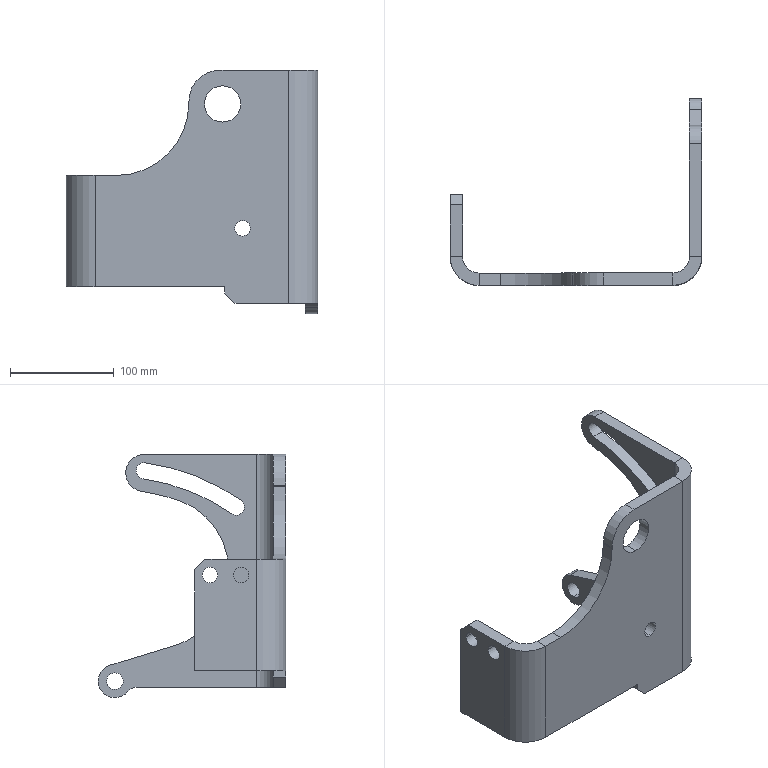Part | SolidWorks | features ICE 3, Chamfer 1, Fillet 1, FlatPattern 1, SMBaseFlange 1, SheetMetal 1 | 1 solid | 52 faces | box 243 x 181 x 235 mm | volume 751047 mm3 | cylinder 27 | plane 25 | commonest cylinder face diameters 15 x6 15.7 x3 32 x3 140 x3 16 x2 35 x2
STEP:
#1=CARTESIAN_POINT('',(12.,-7.5,118.5));
#2=VERTEX_POINT('',#1);
#3=CARTESIAN_POINT('',(12.,-22.5,118.5));
#4=VERTEX_POINT('',#3);
#5=CARTESIAN_POINT('',(12.,-15.,118.5));
#6=DIRECTION('',(-1.,0.,0.));
#7=DIRECTION('',(0.,1.,0.));
#8=AXIS2_PLACEMENT_3D('',#5,#6,#7);
#9=CIRCLE('',#8,7.5);
#10=EDGE_CURVE('',#2,#4,#9,.T.);
#11=ORIENTED_EDGE('',*,*,#10,.F.);
#12=CARTESIAN_POINT('',(0.,-7.5,118.5));
#13=VERTEX_POINT('',#12);
#14=CARTESIAN_POINT('',(243.001,-7.5,118.5));
#15=DIRECTION('',(-1.,0.,0.));
#16=VECTOR('',#15,1000.);
#17=LINE('',#14,#16);
#18=EDGE_CURVE('',#2,#13,#17,.T.);
#19=ORIENTED_EDGE('',*,*,#18,.T.);
#20=CARTESIAN_POINT('',(0.,-22.5,118.5));
#21=VERTEX_POINT('',#20);
#22=CARTESIAN_POINT('',(0.,-15.,118.5));
#23=DIRECTION('',(-1.,0.,0.));
#24=DIRECTION('',(0.,-1.,0.));
#25=AXIS2_PLACEMENT_3D('',#22,#23,#24);
#26=CIRCLE('',#25,7.5);
#27=EDGE_CURVE('',#13,#21,#26,.T.);
#28=ORIENTED_EDGE('',*,*,#27,.T.);
#29=CARTESIAN_POINT('',(243.001,-22.5,118.5));
#30=DIRECTION('',(-1.,0.,0.));
#31=VECTOR('',#30,1000.);
#32=LINE('',#29,#31);
#33=EDGE_CURVE('',#4,#21,#32,.T.);
#34=ORIENTED_EDGE('',*,*,#33,.F.);
#35=EDGE_LOOP('',(#11,#19,#28,#34));
#36=FACE_OUTER_BOUND('',#35,.T.);
#37=CARTESIAN_POINT('',(243.001,-15.,118.5));
#38=DIRECTION('',(-1.,0.,0.));
#39=DIRECTION('',(0.,-1.,0.));
#40=AXIS2_PLACEMENT_3D('',#37,#38,#39);
#41=CYLINDRICAL_SURFACE('',#40,7.5);
#42=ADVANCED_FACE('',(#36),#41,.F.);
#43=CARTESIAN_POINT('',(12.,-37.5,118.5));
#44=VERTEX_POINT('',#43);
#45=CARTESIAN_POINT('',(12.,-52.5,118.5));
#46=VERTEX_POINT('',#45);
#47=CARTESIAN_POINT('',(12.,-45.,118.5));
#48=DIRECTION('',(-1.,0.,0.));
#49=DIRECTION('',(0.,1.,0.));
#50=AXIS2_PLACEMENT_3D('',#47,#48,#49);
#51=CIRCLE('',#50,7.5);
#52=EDGE_CURVE('',#44,#46,#51,.T.);
#53=ORIENTED_EDGE('',*,*,#52,.F.);
#54=CARTESIAN_POINT('',(0.,-37.5,118.5));
#55=VERTEX_POINT('',#54);
#56=CARTESIAN_POINT('',(243.001,-37.5,118.5));
#57=DIRECTION('',(-1.,0.,0.));
#58=VECTOR('',#57,1000.);
#59=LINE('',#56,#58);
#60=EDGE_CURVE('',#44,#55,#59,.T.);
#61=ORIENTED_EDGE('',*,*,#60,.T.);
#62=CARTESIAN_POINT('',(0.,-52.5,118.5));
#63=VERTEX_POINT('',#62);
#64=CARTESIAN_POINT('',(0.,-45.,118.5));
#65=DIRECTION('',(-1.,0.,0.));
#66=DIRECTION('',(0.,-1.,0.));
#67=AXIS2_PLACEMENT_3D('',#64,#65,#66);
#68=CIRCLE('',#67,7.5);
#69=EDGE_CURVE('',#55,#63,#68,.T.);
#70=ORIENTED_EDGE('',*,*,#69,.T.);
#71=CARTESIAN_POINT('',(243.001,-52.5,118.5));
#72=DIRECTION('',(-1.,0.,0.));
#73=VECTOR('',#72,1000.);
#74=LINE('',#71,#73);
#75=EDGE_CURVE('',#46,#63,#74,.T.);
#76=ORIENTED_EDGE('',*,*,#75,.F.);
#77=EDGE_LOOP('',(#53,#61,#70,#76));
#78=FACE_OUTER_BOUND('',#77,.T.);
#79=CARTESIAN_POINT('',(243.001,-45.,118.5));
#80=DIRECTION('',(-1.,0.,0.));
#81=DIRECTION('',(0.,-1.,0.));
#82=AXIS2_PLACEMENT_3D('',#79,#80,#81);
#83=CYLINDRICAL_SURFACE('',#82,7.5);
#84=ADVANCED_FACE('',(#78),#83,.F.);
#85=CARTESIAN_POINT('',(170.4,-88.,90.));
#86=VERTEX_POINT('',#85);
#87=CARTESIAN_POINT('',(170.4,-88.,75.));
#88=VERTEX_POINT('',#87);
#89=CARTESIAN_POINT('',(170.4,-88.,82.5));
#90=DIRECTION('',(0.,-1.,0.));
#91=DIRECTION('',(0.,0.,1.));
#92=AXIS2_PLACEMENT_3D('',#89,#90,#91);
#93=CIRCLE('',#92,7.5);
#94=EDGE_CURVE('',#86,#88,#93,.T.);
#95=ORIENTED_EDGE('',*,*,#94,.T.);
#96=CARTESIAN_POINT('',(170.4,-76.,75.));
#97=VERTEX_POINT('',#96);
#98=CARTESIAN_POINT('',(170.4,-76.,75.));
#99=DIRECTION('',(0.,1.,0.));
#100=VECTOR('',#99,1000.);
#101=LINE('',#98,#100);
#102=EDGE_CURVE('',#88,#97,#101,.T.);
#103=ORIENTED_EDGE('',*,*,#102,.T.);
#104=CARTESIAN_POINT('',(170.4,-76.,90.));
#105=VERTEX_POINT('',#104);
#106=CARTESIAN_POINT('',(170.4,-76.,82.5));
#107=DIRECTION('',(0.,-1.,0.));
#108=DIRECTION('',(0.,0.,1.));
#109=AXIS2_PLACEMENT_3D('',#106,#107,#108);
#110=CIRCLE('',#109,7.5);
#111=EDGE_CURVE('',#105,#97,#110,.T.);
#112=ORIENTED_EDGE('',*,*,#111,.F.);
#113=CARTESIAN_POINT('',(170.4,-76.,90.));
#114=DIRECTION('',(0.,1.,0.));
#115=VECTOR('',#114,1000.);
#116=LINE('',#113,#115);
#117=EDGE_CURVE('',#86,#105,#116,.T.);
#118=ORIENTED_EDGE('',*,*,#117,.F.);
#119=EDGE_LOOP('',(#95,#103,#112,#118));
#120=FACE_OUTER_BOUND('',#119,.T.);
#121=CARTESIAN_POINT('',(170.4,-76.,82.5));
#122=DIRECTION('',(0.,1.,0.));
#123=DIRECTION('',(0.,0.,1.));
#124=AXIS2_PLACEMENT_3D('',#121,#122,#123);
#125=CYLINDRICAL_SURFACE('',#124,7.5);
#126=ADVANCED_FACE('',(#120),#125,.F.);
#127=CARTESIAN_POINT('',(151.,-88.,220.));
#128=VERTEX_POINT('',#127);
#129=CARTESIAN_POINT('',(151.,-88.,185.));
#130=VERTEX_POINT('',#129);
#131=CARTESIAN_POINT('',(151.,-88.,202.5));
#132=DIRECTION('',(0.,-1.,0.));
#133=DIRECTION('',(0.,0.,1.));
#134=AXIS2_PLACEMENT_3D('',#131,#132,#133);
#135=CIRCLE('',#134,17.5);
#136=EDGE_CURVE('',#128,#130,#135,.T.);
#137=ORIENTED_EDGE('',*,*,#136,.T.);
#138=CARTESIAN_POINT('',(151.,-76.,185.));
#139=VERTEX_POINT('',#138);
#140=CARTESIAN_POINT('',(151.,-76.,185.));
#141=DIRECTION('',(0.,1.,0.));
#142=VECTOR('',#141,1000.);
#143=LINE('',#140,#142);
#144=EDGE_CURVE('',#130,#139,#143,.T.);
#145=ORIENTED_EDGE('',*,*,#144,.T.);
#146=CARTESIAN_POINT('',(151.,-76.,220.));
#147=VERTEX_POINT('',#146);
#148=CARTESIAN_POINT('',(151.,-76.,202.5));
#149=DIRECTION('',(0.,-1.,0.));
#150=DIRECTION('',(0.,0.,1.));
#151=AXIS2_PLACEMENT_3D('',#148,#149,#150);
#152=CIRCLE('',#151,17.5);
#153=EDGE_CURVE('',#147,#139,#152,.T.);
#154=ORIENTED_EDGE('',*,*,#153,.F.);
#155=CARTESIAN_POINT('',(151.,-76.,220.));
#156=DIRECTION('',(0.,1.,0.));
#157=VECTOR('',#156,1000.);
#158=LINE('',#155,#157);
#159=EDGE_CURVE('',#128,#147,#158,.T.);
#160=ORIENTED_EDGE('',*,*,#159,.F.);
#161=EDGE_LOOP('',(#137,#145,#154,#160));
#162=FACE_OUTER_BOUND('',#161,.T.);
#163=CARTESIAN_POINT('',(151.,-76.,202.5));
#164=DIRECTION('',(0.,1.,0.));
#165=DIRECTION('',(0.,0.,1.));
#166=AXIS2_PLACEMENT_3D('',#163,#164,#165);
#167=CYLINDRICAL_SURFACE('',#166,17.5);
#168=ADVANCED_FACE('',(#162),#167,.F.);
#169=CARTESIAN_POINT('',(243.,49.591,211.235));
#170=VERTEX_POINT('',#169);
#171=CARTESIAN_POINT('',(243.,48.5,226.859));
#172=VERTEX_POINT('',#171);
#173=CARTESIAN_POINT('',(243.,48.5,219.009));
#174=DIRECTION('',(1.,0.,0.));
#175=DIRECTION('',(0.,0.,1.));
#176=AXIS2_PLACEMENT_3D('',#173,#174,#175);
#177=CIRCLE('',#176,7.85);
#178=EDGE_CURVE('',#170,#172,#177,.T.);
#179=ORIENTED_EDGE('',*,*,#178,.T.);
#180=CARTESIAN_POINT('',(231.,48.5,226.859));
#181=VERTEX_POINT('',#180);
#182=CARTESIAN_POINT('',(231.,48.5,226.859));
#183=DIRECTION('',(-1.,0.,0.));
#184=VECTOR('',#183,1000.);
#185=LINE('',#182,#184);
#186=EDGE_CURVE('',#172,#181,#185,.T.);
#187=ORIENTED_EDGE('',*,*,#186,.T.);
#188=CARTESIAN_POINT('',(231.,49.591,211.235));
#189=VERTEX_POINT('',#188);
#190=CARTESIAN_POINT('',(231.,48.5,219.009));
#191=DIRECTION('',(1.,0.,0.));
#192=DIRECTION('',(0.,0.,1.));
#193=AXIS2_PLACEMENT_3D('',#190,#191,#192);
#194=CIRCLE('',#193,7.85);
#195=EDGE_CURVE('',#189,#181,#194,.T.);
#196=ORIENTED_EDGE('',*,*,#195,.F.);
#197=CARTESIAN_POINT('',(231.,49.591,211.235));
#198=DIRECTION('',(1.,0.,0.));
#199=VECTOR('',#198,1000.);
#200=LINE('',#197,#199);
#201=EDGE_CURVE('',#189,#170,#200,.T.);
#202=ORIENTED_EDGE('',*,*,#201,.T.);
#203=EDGE_LOOP('',(#179,#187,#196,#202));
#204=FACE_OUTER_BOUND('',#203,.T.);
#205=CARTESIAN_POINT('',(231.,48.5,219.009));
#206=DIRECTION('',(-1.,0.,0.));
#207=DIRECTION('',(0.,0.,1.));
#208=AXIS2_PLACEMENT_3D('',#205,#206,#207);
#209=CYLINDRICAL_SURFACE('',#208,7.85);
#210=ADVANCED_FACE('',(#204),#209,.F.);
#211=CARTESIAN_POINT('',(243.,77.,24.));
#212=VERTEX_POINT('',#211);
#213=CARTESIAN_POINT('',(243.,77.,8.));
#214=VERTEX_POINT('',#213);
#215=CARTESIAN_POINT('',(243.,77.,16.));
#216=DIRECTION('',(1.,0.,0.));
#217=DIRECTION('',(0.,0.,1.));
#218=AXIS2_PLACEMENT_3D('',#215,#216,#217);
#219=CIRCLE('',#218,8.);
#220=EDGE_CURVE('',#212,#214,#219,.T.);
#221=ORIENTED_EDGE('',*,*,#220,.T.);
#222=CARTESIAN_POINT('',(231.,77.,8.));
#223=VERTEX_POINT('',#222);
#224=CARTESIAN_POINT('',(231.,77.,8.));
#225=DIRECTION('',(-1.,0.,0.));
#226=VECTOR('',#225,1000.);
#227=LINE('',#224,#226);
#228=EDGE_CURVE('',#214,#223,#227,.T.);
#229=ORIENTED_EDGE('',*,*,#228,.T.);
#230=CARTESIAN_POINT('',(231.,77.,24.));
#231=VERTEX_POINT('',#230);
#232=CARTESIAN_POINT('',(231.,77.,16.));
#233=DIRECTION('',(1.,0.,0.));
#234=DIRECTION('',(0.,0.,1.));
#235=AXIS2_PLACEMENT_3D('',#232,#233,#234);
#236=CIRCLE('',#235,8.);
#237=EDGE_CURVE('',#231,#223,#236,.T.);
#238=ORIENTED_EDGE('',*,*,#237,.F.);
#239=CARTESIAN_POINT('',(231.,77.,24.));
#240=DIRECTION('',(-1.,0.,0.));
#241=VECTOR('',#240,1000.);
#242=LINE('',#239,#241);
#243=EDGE_CURVE('',#212,#231,#242,.T.);
#244=ORIENTED_EDGE('',*,*,#243,.F.);
#245=EDGE_LOOP('',(#221,#229,#238,#244));
#246=FACE_OUTER_BOUND('',#245,.T.);
#247=CARTESIAN_POINT('',(231.,77.,16.));
#248=DIRECTION('',(-1.,0.,0.));
#249=DIRECTION('',(0.,0.,1.));
#250=AXIS2_PLACEMENT_3D('',#247,#248,#249);
#251=CYLINDRICAL_SURFACE('',#250,8.);
#252=ADVANCED_FACE('',(#246),#251,.F.);
#253=CARTESIAN_POINT('',(28.,-76.,133.5));
#254=VERTEX_POINT('',#253);
#255=CARTESIAN_POINT('',(28.,-76.,26.));
#256=VERTEX_POINT('',#255);
#257=CARTESIAN_POINT('',(28.,-76.,235.));
#258=DIRECTION('',(0.,0.,-1.));
#259=VECTOR('',#258,1000.);
#260=LINE('',#257,#259);
#261=EDGE_CURVE('',#254,#256,#260,.T.);
#262=ORIENTED_EDGE('',*,*,#261,.T.);
#263=CARTESIAN_POINT('',(12.,-60.,26.));
#264=VERTEX_POINT('',#263);
#265=CARTESIAN_POINT('',(28.,-60.,26.));
#266=DIRECTION('',(0.,0.,-1.));
#267=DIRECTION('',(-1.,0.,0.));
#268=AXIS2_PLACEMENT_3D('',#265,#266,#267);
#269=CIRCLE('',#268,16.);
#270=EDGE_CURVE('',#256,#264,#269,.T.);
#271=ORIENTED_EDGE('',*,*,#270,.T.);
#272=CARTESIAN_POINT('',(12.,-60.,133.5));
#273=VERTEX_POINT('',#272);
#274=CARTESIAN_POINT('',(12.,-60.,235.));
#275=DIRECTION('',(0.,0.,-1.));
#276=VECTOR('',#275,1000.);
#277=LINE('',#274,#276);
#278=EDGE_CURVE('',#273,#264,#277,.T.);
#279=ORIENTED_EDGE('',*,*,#278,.F.);
#280=CARTESIAN_POINT('',(28.,-60.,133.5));
#281=DIRECTION('',(0.,0.,1.));
#282=DIRECTION('',(-1.,0.,0.));
#283=AXIS2_PLACEMENT_3D('',#280,#281,#282);
#284=CIRCLE('',#283,16.);
#285=EDGE_CURVE('',#273,#254,#284,.T.);
#286=ORIENTED_EDGE('',*,*,#285,.T.);
#287=EDGE_LOOP('',(#262,#271,#279,#286));
#288=FACE_OUTER_BOUND('',#287,.T.);
#289=CARTESIAN_POINT('',(28.,-60.,235.));
#290=DIRECTION('',(0.,0.,-1.));
#291=DIRECTION('',(-1.,0.,0.));
#292=AXIS2_PLACEMENT_3D('',#289,#290,#291);
#293=CYLINDRICAL_SURFACE('',#292,16.);
#294=ADVANCED_FACE('',(#288),#293,.F.);
#295=CARTESIAN_POINT('',(12.,-15.,118.5));
#296=DIRECTION('',(-1.,0.,0.));
#297=DIRECTION('',(0.,1.,0.));
#298=AXIS2_PLACEMENT_3D('',#295,#296,#297);
#299=CIRCLE('',#298,7.5);
#300=EDGE_CURVE('',#4,#2,#299,.T.);
#301=ORIENTED_EDGE('',*,*,#300,.T.);
#302=ORIENTED_EDGE('',*,*,#10,.T.);
#303=EDGE_LOOP('',(#301,#302));
#304=FACE_BOUND('',#303,.T.);
#305=CARTESIAN_POINT('',(12.,-45.,118.5));
#306=DIRECTION('',(-1.,0.,0.));
#307=DIRECTION('',(0.,1.,0.));
#308=AXIS2_PLACEMENT_3D('',#305,#306,#307);
#309=CIRCLE('',#308,7.5);
#310=EDGE_CURVE('',#46,#44,#309,.T.);
#311=ORIENTED_EDGE('',*,*,#310,.T.);
#312=ORIENTED_EDGE('',*,*,#52,.T.);
#313=EDGE_LOOP('',(#311,#312));
#314=FACE_BOUND('',#313,.T.);
#315=CARTESIAN_POINT('',(12.,0.,123.5));
#316=VERTEX_POINT('',#315);
#317=CARTESIAN_POINT('',(12.,0.,26.));
#318=VERTEX_POINT('',#317);
#319=CARTESIAN_POINT('',(12.,0.,235.));
#320=DIRECTION('',(0.,0.,-1.));
#321=VECTOR('',#320,1000.);
#322=LINE('',#319,#321);
#323=EDGE_CURVE('',#316,#318,#322,.T.);
#324=ORIENTED_EDGE('',*,*,#323,.F.);
#325=CARTESIAN_POINT('',(12.,-10.,133.5));
#326=VERTEX_POINT('',#325);
#327=CARTESIAN_POINT('',(12.,-55.75,179.25));
#328=DIRECTION('',(0.,-0.7071,0.7071));
#329=VECTOR('',#328,1000.);
#330=LINE('',#327,#329);
#331=EDGE_CURVE('',#316,#326,#330,.T.);
#332=ORIENTED_EDGE('',*,*,#331,.T.);
#333=CARTESIAN_POINT('',(12.,0.,133.5));
#334=DIRECTION('',(0.,-1.,0.));
#335=VECTOR('',#334,1000.);
#336=LINE('',#333,#335);
#337=EDGE_CURVE('',#326,#273,#336,.T.);
#338=ORIENTED_EDGE('',*,*,#337,.T.);
#339=ORIENTED_EDGE('',*,*,#278,.T.);
#340=CARTESIAN_POINT('',(12.,93.001,26.));
#341=DIRECTION('',(0.,1.,0.));
#342=VECTOR('',#341,1000.);
#343=LINE('',#340,#342);
#344=EDGE_CURVE('',#264,#318,#343,.T.);
#345=ORIENTED_EDGE('',*,*,#344,.T.);
#346=EDGE_LOOP('',(#324,#332,#338,#339,#345));
#347=FACE_OUTER_BOUND('',#346,.T.);
#348=CARTESIAN_POINT('',(12.,0.,235.));
#349=DIRECTION('',(1.,0.,0.));
#350=DIRECTION('',(0.,1.,0.));
#351=AXIS2_PLACEMENT_3D('',#348,#349,#350);
#352=PLANE('',#351);
#353=ADVANCED_FACE('',(#304,#314,#347),#352,.T.);
#354=CARTESIAN_POINT('',(0.,0.,123.5));
#355=VERTEX_POINT('',#354);
#356=CARTESIAN_POINT('',(0.,0.,26.));
#357=VERTEX_POINT('',#356);
#358=CARTESIAN_POINT('',(0.,0.,235.));
#359=DIRECTION('',(0.,0.,-1.));
#360=VECTOR('',#359,1000.);
#361=LINE('',#358,#360);
#362=EDGE_CURVE('',#355,#357,#361,.T.);
#363=ORIENTED_EDGE('',*,*,#362,.F.);
#364=CARTESIAN_POINT('',(0.,0.,123.5));
#365=DIRECTION('',(1.,0.,0.));
#366=VECTOR('',#365,1000.);
#367=LINE('',#364,#366);
#368=EDGE_CURVE('',#355,#316,#367,.T.);
#369=ORIENTED_EDGE('',*,*,#368,.T.);
#370=ORIENTED_EDGE('',*,*,#323,.T.);
#371=CARTESIAN_POINT('',(12.,0.,26.));
#372=DIRECTION('',(-1.,0.,0.));
#373=VECTOR('',#372,1000.);
#374=LINE('',#371,#373);
#375=EDGE_CURVE('',#318,#357,#374,.T.);
#376=ORIENTED_EDGE('',*,*,#375,.T.);
#377=EDGE_LOOP('',(#363,#369,#370,#376));
#378=FACE_OUTER_BOUND('',#377,.T.);
#379=CARTESIAN_POINT('',(0.,0.,235.));
#380=DIRECTION('',(0.,1.,0.));
#381=DIRECTION('',(-1.,0.,0.));
#382=AXIS2_PLACEMENT_3D('',#379,#380,#381);
#383=PLANE('',#382);
#384=ADVANCED_FACE('',(#378),#383,.T.);
#385=CARTESIAN_POINT('',(0.,-15.,118.5));
#386=DIRECTION('',(-1.,0.,0.));
#387=DIRECTION('',(0.,-1.,0.));
#388=AXIS2_PLACEMENT_3D('',#385,#386,#387);
#389=CIRCLE('',#388,7.5);
#390=EDGE_CURVE('',#21,#13,#389,.T.);
#391=ORIENTED_EDGE('',*,*,#390,.F.);
#392=ORIENTED_EDGE('',*,*,#27,.F.);
#393=EDGE_LOOP('',(#391,#392));
#394=FACE_BOUND('',#393,.T.);
#395=CARTESIAN_POINT('',(0.,-45.,118.5));
#396=DIRECTION('',(-1.,0.,0.));
#397=DIRECTION('',(0.,-1.,0.));
#398=AXIS2_PLACEMENT_3D('',#395,#396,#397);
#399=CIRCLE('',#398,7.5);
#400=EDGE_CURVE('',#63,#55,#399,.T.);
#401=ORIENTED_EDGE('',*,*,#400,.F.);
#402=ORIENTED_EDGE('',*,*,#69,.F.);
#403=EDGE_LOOP('',(#401,#402));
#404=FACE_BOUND('',#403,.T.);
#405=CARTESIAN_POINT('',(0.,-10.,133.5));
#406=VERTEX_POINT('',#405);
#407=CARTESIAN_POINT('',(0.,-60.,133.5));
#408=VERTEX_POINT('',#407);
#409=CARTESIAN_POINT('',(0.,93.001,133.5));
#410=DIRECTION('',(0.,-1.,0.));
#411=VECTOR('',#410,1000.);
#412=LINE('',#409,#411);
#413=EDGE_CURVE('',#406,#408,#412,.T.);
#414=ORIENTED_EDGE('',*,*,#413,.F.);
#415=CARTESIAN_POINT('',(0.,0.,123.5));
#416=DIRECTION('',(0.,0.7071,-0.7071));
#417=VECTOR('',#416,1000.);
#418=LINE('',#415,#417);
#419=EDGE_CURVE('',#406,#355,#418,.T.);
#420=ORIENTED_EDGE('',*,*,#419,.T.);
#421=ORIENTED_EDGE('',*,*,#362,.T.);
#422=CARTESIAN_POINT('',(0.,-60.,26.));
#423=VERTEX_POINT('',#422);
#424=CARTESIAN_POINT('',(0.,0.,26.));
#425=DIRECTION('',(0.,1.,0.));
#426=VECTOR('',#425,1000.);
#427=LINE('',#424,#426);
#428=EDGE_CURVE('',#423,#357,#427,.T.);
#429=ORIENTED_EDGE('',*,*,#428,.F.);
#430=CARTESIAN_POINT('',(0.,-60.,235.));
#431=DIRECTION('',(0.,0.,-1.));
#432=VECTOR('',#431,1000.);
#433=LINE('',#430,#432);
#434=EDGE_CURVE('',#408,#423,#433,.T.);
#435=ORIENTED_EDGE('',*,*,#434,.F.);
#436=EDGE_LOOP('',(#414,#420,#421,#429,#435));
#437=FACE_OUTER_BOUND('',#436,.T.);
#438=CARTESIAN_POINT('',(0.,0.,235.));
#439=DIRECTION('',(1.,0.,0.));
#440=DIRECTION('',(0.,1.,0.));
#441=AXIS2_PLACEMENT_3D('',#438,#439,#440);
#442=PLANE('',#441);
#443=ADVANCED_FACE('',(#394,#404,#437),#442,.F.);
#444=CARTESIAN_POINT('',(28.,-88.,26.));
#445=VERTEX_POINT('',#444);
#446=CARTESIAN_POINT('',(28.,-60.,26.));
#447=DIRECTION('',(0.,0.,-1.));
#448=DIRECTION('',(1.,0.,0.));
#449=AXIS2_PLACEMENT_3D('',#446,#447,#448);
#450=CIRCLE('',#449,28.);
#451=EDGE_CURVE('',#445,#423,#450,.T.);
#452=ORIENTED_EDGE('',*,*,#451,.F.);
#453=CARTESIAN_POINT('',(28.,-88.,133.5));
#454=VERTEX_POINT('',#453);
#455=CARTESIAN_POINT('',(28.,-88.,235.));
#456=DIRECTION('',(0.,0.,-1.));
#457=VECTOR('',#456,1000.);
#458=LINE('',#455,#457);
#459=EDGE_CURVE('',#454,#445,#458,.T.);
#460=ORIENTED_EDGE('',*,*,#459,.F.);
#461=CARTESIAN_POINT('',(28.,-60.,133.5));
#462=DIRECTION('',(0.,0.,1.));
#463=DIRECTION('',(-1.,0.,0.));
#464=AXIS2_PLACEMENT_3D('',#461,#462,#463);
#465=CIRCLE('',#464,28.);
#466=EDGE_CURVE('',#408,#454,#465,.T.);
#467=ORIENTED_EDGE('',*,*,#466,.F.);
#468=ORIENTED_EDGE('',*,*,#434,.T.);
#469=EDGE_LOOP('',(#452,#460,#467,#468));
#470=FACE_OUTER_BOUND('',#469,.T.);
#471=CARTESIAN_POINT('',(28.,-60.,235.));
#472=DIRECTION('',(0.,0.,-1.));
#473=DIRECTION('',(-1.,0.,0.));
#474=AXIS2_PLACEMENT_3D('',#471,#472,#473);
#475=CYLINDRICAL_SURFACE('',#474,28.);
#476=ADVANCED_FACE('',(#470),#475,.T.);
#477=CARTESIAN_POINT('',(243.,-35.904,177.619));
#478=VERTEX_POINT('',#477);
#479=CARTESIAN_POINT('',(243.,77.,16.));
#480=DIRECTION('',(1.,0.,0.));
#481=DIRECTION('',(0.,0.,1.));
#482=AXIS2_PLACEMENT_3D('',#479,#480,#481);
#483=CIRCLE('',#482,197.15);
#484=EDGE_CURVE('',#170,#478,#483,.T.);
#485=ORIENTED_EDGE('',*,*,#484,.T.);
#486=CARTESIAN_POINT('',(243.,-44.896,190.49));
#487=VERTEX_POINT('',#486);
#488=CARTESIAN_POINT('',(243.,-40.4,184.054));
#489=DIRECTION('',(1.,0.,0.));
#490=DIRECTION('',(0.,0.,1.));
#491=AXIS2_PLACEMENT_3D('',#488,#489,#490);
#492=CIRCLE('',#491,7.85);
#493=EDGE_CURVE('',#487,#478,#492,.T.);
#494=ORIENTED_EDGE('',*,*,#493,.F.);
#495=CARTESIAN_POINT('',(243.,47.409,226.783));
#496=VERTEX_POINT('',#495);
#497=CARTESIAN_POINT('',(243.,77.,16.));
#498=DIRECTION('',(1.,0.,0.));
#499=DIRECTION('',(0.,0.,1.));
#500=AXIS2_PLACEMENT_3D('',#497,#498,#499);
#501=CIRCLE('',#500,212.85);
#502=EDGE_CURVE('',#496,#487,#501,.T.);
#503=ORIENTED_EDGE('',*,*,#502,.F.);
#504=CARTESIAN_POINT('',(243.,48.5,219.009));
#505=DIRECTION('',(1.,0.,0.));
#506=DIRECTION('',(0.,0.,1.));
#507=AXIS2_PLACEMENT_3D('',#504,#505,#506);
#508=CIRCLE('',#507,7.85);
#509=EDGE_CURVE('',#172,#496,#508,.T.);
#510=ORIENTED_EDGE('',*,*,#509,.F.);
#511=ORIENTED_EDGE('',*,*,#178,.F.);
#512=EDGE_LOOP('',(#485,#494,#503,#510,#511));
#513=FACE_BOUND('',#512,.T.);
#514=ORIENTED_EDGE('',*,*,#220,.F.);
#515=CARTESIAN_POINT('',(243.,77.,16.));
#516=DIRECTION('',(1.,0.,0.));
#517=DIRECTION('',(0.,0.,1.));
#518=AXIS2_PLACEMENT_3D('',#515,#516,#517);
#519=CIRCLE('',#518,8.);
#520=EDGE_CURVE('',#214,#212,#519,.T.);
#521=ORIENTED_EDGE('',*,*,#520,.F.);
#522=EDGE_LOOP('',(#514,#521));
#523=FACE_BOUND('',#522,.T.);
#524=CARTESIAN_POINT('',(243.,64.388,6.154));
#525=VERTEX_POINT('',#524);
#526=CARTESIAN_POINT('',(243.,81.671,31.303));
#527=VERTEX_POINT('',#526);
#528=CARTESIAN_POINT('',(243.,77.,16.));
#529=DIRECTION('',(1.,0.,0.));
#530=DIRECTION('',(0.,0.,1.));
#531=AXIS2_PLACEMENT_3D('',#528,#529,#530);
#532=CIRCLE('',#531,16.);
#533=EDGE_CURVE('',#525,#527,#532,.T.);
#534=ORIENTED_EDGE('',*,*,#533,.T.);
#535=CARTESIAN_POINT('',(243.,18.453,50.601));
#536=VERTEX_POINT('',#535);
#537=CARTESIAN_POINT('',(243.,15.703,51.44));
#538=DIRECTION('',(0.,-0.9564,0.292));
#539=VECTOR('',#538,1000.);
#540=LINE('',#537,#539);
#541=EDGE_CURVE('',#527,#536,#540,.T.);
#542=ORIENTED_EDGE('',*,*,#541,.T.);
#543=CARTESIAN_POINT('',(243.,-29.309,101.774));
#544=VERTEX_POINT('',#543);
#545=CARTESIAN_POINT('',(243.,38.89,117.551));
#546=DIRECTION('',(-1.,0.,0.));
#547=DIRECTION('',(0.,0.,1.));
#548=AXIS2_PLACEMENT_3D('',#545,#546,#547);
#549=CIRCLE('',#548,70.);
#550=EDGE_CURVE('',#536,#544,#549,.T.);
#551=ORIENTED_EDGE('',*,*,#550,.T.);
#552=CARTESIAN_POINT('',(243.,-30.797,108.208));
#553=VERTEX_POINT('',#552);
#554=CARTESIAN_POINT('',(243.,-5.472,-1.266));
#555=DIRECTION('',(0.,-0.2254,0.9743));
#556=VECTOR('',#555,1000.);
#557=LINE('',#554,#556);
#558=EDGE_CURVE('',#544,#553,#557,.T.);
#559=ORIENTED_EDGE('',*,*,#558,.T.);
#560=CARTESIAN_POINT('',(243.,13.302,189.705));
#561=VERTEX_POINT('',#560);
#562=CARTESIAN_POINT('',(243.,37.402,123.985));
#563=DIRECTION('',(-1.,0.,0.));
#564=DIRECTION('',(0.,0.,1.));
#565=AXIS2_PLACEMENT_3D('',#562,#563,#564);
#566=CIRCLE('',#565,70.);
#567=EDGE_CURVE('',#553,#561,#566,.T.);
#568=ORIENTED_EDGE('',*,*,#567,.T.);
#569=CARTESIAN_POINT('',(243.,50.992,199.179));
#570=VERTEX_POINT('',#569);
#571=CARTESIAN_POINT('',(243.,77.,16.));
#572=DIRECTION('',(1.,0.,0.));
#573=DIRECTION('',(0.,0.,1.));
#574=AXIS2_PLACEMENT_3D('',#571,#572,#573);
#575=CIRCLE('',#574,185.016);
#576=EDGE_CURVE('',#570,#561,#575,.T.);
#577=ORIENTED_EDGE('',*,*,#576,.F.);
#578=CARTESIAN_POINT('',(243.,48.461,235.));
#579=VERTEX_POINT('',#578);
#580=CARTESIAN_POINT('',(243.,48.461,217.));
#581=DIRECTION('',(1.,0.,0.));
#582=DIRECTION('',(0.,0.,1.));
#583=AXIS2_PLACEMENT_3D('',#580,#581,#582);
#584=CIRCLE('',#583,18.);
#585=EDGE_CURVE('',#570,#579,#584,.T.);
#586=ORIENTED_EDGE('',*,*,#585,.T.);
#587=CARTESIAN_POINT('',(243.,-60.,235.));
#588=VERTEX_POINT('',#587);
#589=CARTESIAN_POINT('',(243.,-88.,235.));
#590=DIRECTION('',(0.,1.,0.));
#591=VECTOR('',#590,1000.);
#592=LINE('',#589,#591);
#593=EDGE_CURVE('',#588,#579,#592,.T.);
#594=ORIENTED_EDGE('',*,*,#593,.F.);
#595=CARTESIAN_POINT('',(243.,-60.,10.));
#596=VERTEX_POINT('',#595);
#597=CARTESIAN_POINT('',(243.,-60.,235.));
#598=DIRECTION('',(0.,0.,-1.));
#599=VECTOR('',#598,1000.);
#600=LINE('',#597,#599);
#601=EDGE_CURVE('',#588,#596,#600,.T.);
#602=ORIENTED_EDGE('',*,*,#601,.T.);
#603=CARTESIAN_POINT('',(243.,56.506,10.));
#604=VERTEX_POINT('',#603);
#605=CARTESIAN_POINT('',(243.,-88.,10.));
#606=DIRECTION('',(0.,1.,0.));
#607=VECTOR('',#606,1000.);
#608=LINE('',#605,#607);
#609=EDGE_CURVE('',#596,#604,#608,.T.);
#610=ORIENTED_EDGE('',*,*,#609,.T.);
#611=CARTESIAN_POINT('',(243.,56.506,0.));
#612=DIRECTION('',(-1.,0.,0.));
#613=DIRECTION('',(0.,0.,1.));
#614=AXIS2_PLACEMENT_3D('',#611,#612,#613);
#615=CIRCLE('',#614,10.);
#616=EDGE_CURVE('',#604,#525,#615,.T.);
#617=ORIENTED_EDGE('',*,*,#616,.T.);
#618=EDGE_LOOP('',(#534,#542,#551,#559,#568,#577,#586,#594,#602,#610,#617));
#619=FACE_OUTER_BOUND('',#618,.T.);
#620=CARTESIAN_POINT('',(243.,-88.,235.));
#621=DIRECTION('',(-1.,0.,0.));
#622=DIRECTION('',(0.,0.,1.));
#623=AXIS2_PLACEMENT_3D('',#620,#621,#622);
#624=PLANE('',#623);
#625=ADVANCED_FACE('',(#513,#523,#619),#624,.F.);
#626=ORIENTED_EDGE('',*,*,#237,.T.);
#627=CARTESIAN_POINT('',(231.,77.,16.));
#628=DIRECTION('',(1.,0.,0.));
#629=DIRECTION('',(0.,0.,1.));
#630=AXIS2_PLACEMENT_3D('',#627,#628,#629);
#631=CIRCLE('',#630,8.);
#632=EDGE_CURVE('',#223,#231,#631,.T.);
#633=ORIENTED_EDGE('',*,*,#632,.T.);
#634=EDGE_LOOP('',(#626,#633));
#635=FACE_BOUND('',#634,.T.);
#636=CARTESIAN_POINT('',(231.,-44.896,190.49));
#637=VERTEX_POINT('',#636);
#638=CARTESIAN_POINT('',(231.,-35.904,177.619));
#639=VERTEX_POINT('',#638);
#640=CARTESIAN_POINT('',(231.,-40.4,184.054));
#641=DIRECTION('',(1.,0.,0.));
#642=DIRECTION('',(0.,0.,1.));
#643=AXIS2_PLACEMENT_3D('',#640,#641,#642);
#644=CIRCLE('',#643,7.85);
#645=EDGE_CURVE('',#637,#639,#644,.T.);
#646=ORIENTED_EDGE('',*,*,#645,.T.);
#647=CARTESIAN_POINT('',(231.,77.,16.));
#648=DIRECTION('',(1.,0.,0.));
#649=DIRECTION('',(0.,0.,1.));
#650=AXIS2_PLACEMENT_3D('',#647,#648,#649);
#651=CIRCLE('',#650,197.15);
#652=EDGE_CURVE('',#189,#639,#651,.T.);
#653=ORIENTED_EDGE('',*,*,#652,.F.);
#654=ORIENTED_EDGE('',*,*,#195,.T.);
#655=CARTESIAN_POINT('',(231.,47.409,226.783));
#656=VERTEX_POINT('',#655);
#657=CARTESIAN_POINT('',(231.,48.5,219.009));
#658=DIRECTION('',(1.,0.,0.));
#659=DIRECTION('',(0.,0.,1.));
#660=AXIS2_PLACEMENT_3D('',#657,#658,#659);
#661=CIRCLE('',#660,7.85);
#662=EDGE_CURVE('',#181,#656,#661,.T.);
#663=ORIENTED_EDGE('',*,*,#662,.T.);
#664=CARTESIAN_POINT('',(231.,77.,16.));
#665=DIRECTION('',(1.,0.,0.));
#666=DIRECTION('',(0.,0.,1.));
#667=AXIS2_PLACEMENT_3D('',#664,#665,#666);
#668=CIRCLE('',#667,212.85);
#669=EDGE_CURVE('',#656,#637,#668,.T.);
#670=ORIENTED_EDGE('',*,*,#669,.T.);
#671=EDGE_LOOP('',(#646,#653,#654,#663,#670));
#672=FACE_BOUND('',#671,.T.);
#673=CARTESIAN_POINT('',(231.,81.671,31.303));
#674=VERTEX_POINT('',#673);
#675=CARTESIAN_POINT('',(231.,18.453,50.601));
#676=VERTEX_POINT('',#675);
#677=CARTESIAN_POINT('',(231.,15.703,51.44));
#678=DIRECTION('',(0.,-0.9564,0.292));
#679=VECTOR('',#678,1000.);
#680=LINE('',#677,#679);
#681=EDGE_CURVE('',#674,#676,#680,.T.);
#682=ORIENTED_EDGE('',*,*,#681,.F.);
#683=CARTESIAN_POINT('',(231.,64.388,6.154));
#684=VERTEX_POINT('',#683);
#685=CARTESIAN_POINT('',(231.,77.,16.));
#686=DIRECTION('',(1.,0.,0.));
#687=DIRECTION('',(0.,0.,1.));
#688=AXIS2_PLACEMENT_3D('',#685,#686,#687);
#689=CIRCLE('',#688,16.);
#690=EDGE_CURVE('',#684,#674,#689,.T.);
#691=ORIENTED_EDGE('',*,*,#690,.F.);
#692=CARTESIAN_POINT('',(231.,56.506,10.));
#693=VERTEX_POINT('',#692);
#694=CARTESIAN_POINT('',(231.,56.506,0.));
#695=DIRECTION('',(-1.,0.,0.));
#696=DIRECTION('',(0.,0.,1.));
#697=AXIS2_PLACEMENT_3D('',#694,#695,#696);
#698=CIRCLE('',#697,10.);
#699=EDGE_CURVE('',#693,#684,#698,.T.);
#700=ORIENTED_EDGE('',*,*,#699,.F.);
#701=CARTESIAN_POINT('',(231.,-60.,10.));
#702=VERTEX_POINT('',#701);
#703=CARTESIAN_POINT('',(231.,0.,10.));
#704=DIRECTION('',(0.,1.,0.));
#705=VECTOR('',#704,1000.);
#706=LINE('',#703,#705);
#707=EDGE_CURVE('',#702,#693,#706,.T.);
#708=ORIENTED_EDGE('',*,*,#707,.F.);
#709=CARTESIAN_POINT('',(231.,-60.,235.));
#710=VERTEX_POINT('',#709);
#711=CARTESIAN_POINT('',(231.,-60.,235.));
#712=DIRECTION('',(0.,0.,-1.));
#713=VECTOR('',#712,1000.);
#714=LINE('',#711,#713);
#715=EDGE_CURVE('',#710,#702,#714,.T.);
#716=ORIENTED_EDGE('',*,*,#715,.F.);
#717=CARTESIAN_POINT('',(231.,48.461,235.));
#718=VERTEX_POINT('',#717);
#719=CARTESIAN_POINT('',(231.,-88.,235.));
#720=DIRECTION('',(0.,1.,0.));
#721=VECTOR('',#720,1000.);
#722=LINE('',#719,#721);
#723=EDGE_CURVE('',#710,#718,#722,.T.);
#724=ORIENTED_EDGE('',*,*,#723,.T.);
#725=CARTESIAN_POINT('',(231.,50.992,199.179));
#726=VERTEX_POINT('',#725);
#727=CARTESIAN_POINT('',(231.,48.461,217.));
#728=DIRECTION('',(1.,0.,0.));
#729=DIRECTION('',(0.,0.,1.));
#730=AXIS2_PLACEMENT_3D('',#727,#728,#729);
#731=CIRCLE('',#730,18.);
#732=EDGE_CURVE('',#726,#718,#731,.T.);
#733=ORIENTED_EDGE('',*,*,#732,.F.);
#734=CARTESIAN_POINT('',(231.,13.302,189.705));
#735=VERTEX_POINT('',#734);
#736=CARTESIAN_POINT('',(231.,77.,16.));
#737=DIRECTION('',(1.,0.,0.));
#738=DIRECTION('',(0.,0.,1.));
#739=AXIS2_PLACEMENT_3D('',#736,#737,#738);
#740=CIRCLE('',#739,185.016);
#741=EDGE_CURVE('',#726,#735,#740,.T.);
#742=ORIENTED_EDGE('',*,*,#741,.T.);
#743=CARTESIAN_POINT('',(231.,-30.797,108.208));
#744=VERTEX_POINT('',#743);
#745=CARTESIAN_POINT('',(231.,37.402,123.985));
#746=DIRECTION('',(-1.,0.,0.));
#747=DIRECTION('',(0.,0.,1.));
#748=AXIS2_PLACEMENT_3D('',#745,#746,#747);
#749=CIRCLE('',#748,70.);
#750=EDGE_CURVE('',#744,#735,#749,.T.);
#751=ORIENTED_EDGE('',*,*,#750,.F.);
#752=CARTESIAN_POINT('',(231.,-29.309,101.774));
#753=VERTEX_POINT('',#752);
#754=CARTESIAN_POINT('',(231.,-5.472,-1.266));
#755=DIRECTION('',(0.,-0.2254,0.9743));
#756=VECTOR('',#755,1000.);
#757=LINE('',#754,#756);
#758=EDGE_CURVE('',#753,#744,#757,.T.);
#759=ORIENTED_EDGE('',*,*,#758,.F.);
#760=CARTESIAN_POINT('',(231.,38.89,117.551));
#761=DIRECTION('',(-1.,0.,0.));
#762=DIRECTION('',(0.,0.,1.));
#763=AXIS2_PLACEMENT_3D('',#760,#761,#762);
#764=CIRCLE('',#763,70.);
#765=EDGE_CURVE('',#676,#753,#764,.T.);
#766=ORIENTED_EDGE('',*,*,#765,.F.);
#767=EDGE_LOOP('',(#682,#691,#700,#708,#716,#724,#733,#742,#751,#759,#766));
#768=FACE_OUTER_BOUND('',#767,.T.);
#769=CARTESIAN_POINT('',(231.,-88.,235.));
#770=DIRECTION('',(-1.,0.,0.));
#771=DIRECTION('',(0.,0.,1.));
#772=AXIS2_PLACEMENT_3D('',#769,#770,#771);
#773=PLANE('',#772);
#774=ADVANCED_FACE('',(#635,#672,#768),#773,.T.);
#775=ORIENTED_EDGE('',*,*,#715,.T.);
#776=CARTESIAN_POINT('',(215.,-76.,10.));
#777=VERTEX_POINT('',#776);
#778=CARTESIAN_POINT('',(215.,-60.,10.));
#779=DIRECTION('',(0.,0.,1.));
#780=DIRECTION('',(-1.,0.,0.));
#781=AXIS2_PLACEMENT_3D('',#778,#779,#780);
#782=CIRCLE('',#781,16.);
#783=EDGE_CURVE('',#777,#702,#782,.T.);
#784=ORIENTED_EDGE('',*,*,#783,.F.);
#785=CARTESIAN_POINT('',(215.,-76.,235.));
#786=VERTEX_POINT('',#785);
#787=CARTESIAN_POINT('',(215.,-76.,235.));
#788=DIRECTION('',(0.,0.,-1.));
#789=VECTOR('',#788,1000.);
#790=LINE('',#787,#789);
#791=EDGE_CURVE('',#786,#777,#790,.T.);
#792=ORIENTED_EDGE('',*,*,#791,.F.);
#793=CARTESIAN_POINT('',(215.,-60.,235.));
#794=DIRECTION('',(0.,0.,1.));
#795=DIRECTION('',(1.,0.,0.));
#796=AXIS2_PLACEMENT_3D('',#793,#794,#795);
#797=CIRCLE('',#796,16.);
#798=EDGE_CURVE('',#786,#710,#797,.T.);
#799=ORIENTED_EDGE('',*,*,#798,.T.);
#800=EDGE_LOOP('',(#775,#784,#792,#799));
#801=FACE_OUTER_BOUND('',#800,.T.);
#802=CARTESIAN_POINT('',(215.,-60.,235.));
#803=DIRECTION('',(0.,0.,-1.));
#804=DIRECTION('',(-1.,0.,0.));
#805=AXIS2_PLACEMENT_3D('',#802,#803,#804);
#806=CYLINDRICAL_SURFACE('',#805,16.);
#807=ADVANCED_FACE('',(#801),#806,.F.);
#808=CARTESIAN_POINT('',(215.,-88.,10.));
#809=VERTEX_POINT('',#808);
#810=CARTESIAN_POINT('',(215.,-60.,10.));
#811=DIRECTION('',(0.,0.,1.));
#812=DIRECTION('',(-1.,0.,0.));
#813=AXIS2_PLACEMENT_3D('',#810,#811,#812);
#814=CIRCLE('',#813,28.);
#815=EDGE_CURVE('',#809,#596,#814,.T.);
#816=ORIENTED_EDGE('',*,*,#815,.T.);
#817=ORIENTED_EDGE('',*,*,#601,.F.);
#818=CARTESIAN_POINT('',(215.,-88.,235.));
#819=VERTEX_POINT('',#818);
#820=CARTESIAN_POINT('',(215.,-60.,235.));
#821=DIRECTION('',(0.,0.,1.));
#822=DIRECTION('',(-1.,0.,0.));
#823=AXIS2_PLACEMENT_3D('',#820,#821,#822);
#824=CIRCLE('',#823,28.);
#825=EDGE_CURVE('',#819,#588,#824,.T.);
#826=ORIENTED_EDGE('',*,*,#825,.F.);
#827=CARTESIAN_POINT('',(215.,-88.,235.));
#828=DIRECTION('',(0.,0.,-1.));
#829=VECTOR('',#828,1000.);
#830=LINE('',#827,#829);
#831=EDGE_CURVE('',#819,#809,#830,.T.);
#832=ORIENTED_EDGE('',*,*,#831,.T.);
#833=EDGE_LOOP('',(#816,#817,#826,#832));
#834=FACE_OUTER_BOUND('',#833,.T.);
#835=CARTESIAN_POINT('',(215.,-60.,235.));
#836=DIRECTION('',(0.,0.,-1.));
#837=DIRECTION('',(-1.,0.,0.));
#838=AXIS2_PLACEMENT_3D('',#835,#836,#837);
#839=CYLINDRICAL_SURFACE('',#838,28.);
#840=ADVANCED_FACE('',(#834),#839,.T.);
#841=ORIENTED_EDGE('',*,*,#593,.T.);
#842=CARTESIAN_POINT('',(231.,48.461,235.));
#843=DIRECTION('',(1.,0.,0.));
#844=VECTOR('',#843,1000.);
#845=LINE('',#842,#844);
#846=EDGE_CURVE('',#718,#579,#845,.T.);
#847=ORIENTED_EDGE('',*,*,#846,.F.);
#848=ORIENTED_EDGE('',*,*,#723,.F.);
#849=CARTESIAN_POINT('',(231.,-60.,235.));
#850=DIRECTION('',(1.,0.,0.));
#851=VECTOR('',#850,1000.);
#852=LINE('',#849,#851);
#853=EDGE_CURVE('',#710,#588,#852,.T.);
#854=ORIENTED_EDGE('',*,*,#853,.T.);
#855=EDGE_LOOP('',(#841,#847,#848,#854));
#856=FACE_OUTER_BOUND('',#855,.T.);
#857=CARTESIAN_POINT('',(215.,-60.,235.));
#858=DIRECTION('',(0.,0.,1.));
#859=DIRECTION('',(1.,0.,0.));
#860=AXIS2_PLACEMENT_3D('',#857,#858,#859);
#861=PLANE('',#860);
#862=ADVANCED_FACE('',(#856),#861,.T.);
#863=ORIENTED_EDGE('',*,*,#111,.T.);
#864=CARTESIAN_POINT('',(170.4,-76.,82.5));
#865=DIRECTION('',(0.,-1.,0.));
#866=DIRECTION('',(0.,0.,1.));
#867=AXIS2_PLACEMENT_3D('',#864,#865,#866);
#868=CIRCLE('',#867,7.5);
#869=EDGE_CURVE('',#97,#105,#868,.T.);
#870=ORIENTED_EDGE('',*,*,#869,.T.);
#871=EDGE_LOOP('',(#863,#870));
#872=FACE_BOUND('',#871,.T.);
#873=ORIENTED_EDGE('',*,*,#153,.T.);
#874=CARTESIAN_POINT('',(151.,-76.,202.5));
#875=DIRECTION('',(0.,-1.,0.));
#876=DIRECTION('',(0.,0.,1.));
#877=AXIS2_PLACEMENT_3D('',#874,#875,#876);
#878=CIRCLE('',#877,17.5);
#879=EDGE_CURVE('',#139,#147,#878,.T.);
#880=ORIENTED_EDGE('',*,*,#879,.T.);
#881=EDGE_LOOP('',(#873,#880));
#882=FACE_BOUND('',#881,.T.);
#883=CARTESIAN_POINT('',(118.5,-76.,203.5));
#884=VERTEX_POINT('',#883);
#885=CARTESIAN_POINT('',(118.5,-76.,205.));
#886=VERTEX_POINT('',#885);
#887=CARTESIAN_POINT('',(118.5,-76.,203.5));
#888=DIRECTION('',(0.,0.,1.));
#889=VECTOR('',#888,1000.);
#890=LINE('',#887,#889);
#891=EDGE_CURVE('',#884,#886,#890,.T.);
#892=ORIENTED_EDGE('',*,*,#891,.T.);
#893=CARTESIAN_POINT('',(148.5,-76.,235.));
#894=VERTEX_POINT('',#893);
#895=CARTESIAN_POINT('',(148.5,-76.,205.));
#896=DIRECTION('',(0.,1.,0.));
#897=DIRECTION('',(0.,0.,1.));
#898=AXIS2_PLACEMENT_3D('',#895,#896,#897);
#899=CIRCLE('',#898,30.);
#900=EDGE_CURVE('',#886,#894,#899,.T.);
#901=ORIENTED_EDGE('',*,*,#900,.T.);
#902=CARTESIAN_POINT('',(0.,-76.,235.));
#903=DIRECTION('',(1.,0.,0.));
#904=VECTOR('',#903,1000.);
#905=LINE('',#902,#904);
#906=EDGE_CURVE('',#894,#786,#905,.T.);
#907=ORIENTED_EDGE('',*,*,#906,.T.);
#908=ORIENTED_EDGE('',*,*,#791,.T.);
#909=CARTESIAN_POINT('',(163.,-76.,10.));
#910=VERTEX_POINT('',#909);
#911=CARTESIAN_POINT('',(-0.001,-76.,10.));
#912=DIRECTION('',(1.,0.,0.));
#913=VECTOR('',#912,1000.);
#914=LINE('',#911,#913);
#915=EDGE_CURVE('',#910,#777,#914,.T.);
#916=ORIENTED_EDGE('',*,*,#915,.F.);
#917=CARTESIAN_POINT('',(153.,-76.,20.));
#918=VERTEX_POINT('',#917);
#919=CARTESIAN_POINT('',(153.,-76.,20.));
#920=DIRECTION('',(-0.7071,0.,0.7071));
#921=VECTOR('',#920,1000.);
#922=LINE('',#919,#921);
#923=EDGE_CURVE('',#910,#918,#922,.T.);
#924=ORIENTED_EDGE('',*,*,#923,.T.);
#925=CARTESIAN_POINT('',(153.,-76.,26.));
#926=VERTEX_POINT('',#925);
#927=CARTESIAN_POINT('',(153.,-76.,26.));
#928=DIRECTION('',(0.,0.,1.));
#929=VECTOR('',#928,1000.);
#930=LINE('',#927,#929);
#931=EDGE_CURVE('',#918,#926,#930,.T.);
#932=ORIENTED_EDGE('',*,*,#931,.T.);
#933=CARTESIAN_POINT('',(0.,-76.,26.));
#934=DIRECTION('',(-1.,0.,0.));
#935=VECTOR('',#934,1000.);
#936=LINE('',#933,#935);
#937=EDGE_CURVE('',#926,#256,#936,.T.);
#938=ORIENTED_EDGE('',*,*,#937,.T.);
#939=ORIENTED_EDGE('',*,*,#261,.F.);
#940=CARTESIAN_POINT('',(48.5,-76.,133.5));
#941=VERTEX_POINT('',#940);
#942=CARTESIAN_POINT('',(0.,-76.,133.5));
#943=DIRECTION('',(1.,0.,0.));
#944=VECTOR('',#943,1000.);
#945=LINE('',#942,#944);
#946=EDGE_CURVE('',#254,#941,#945,.T.);
#947=ORIENTED_EDGE('',*,*,#946,.T.);
#948=CARTESIAN_POINT('',(48.5,-76.,203.5));
#949=DIRECTION('',(0.,-1.,0.));
#950=DIRECTION('',(0.,0.,1.));
#951=AXIS2_PLACEMENT_3D('',#948,#949,#950);
#952=CIRCLE('',#951,70.);
#953=EDGE_CURVE('',#941,#884,#952,.T.);
#954=ORIENTED_EDGE('',*,*,#953,.T.);
#955=EDGE_LOOP('',(#892,#901,#907,#908,#916,#924,#932,#938,#939,#947,#954));
#956=FACE_OUTER_BOUND('',#955,.T.);
#957=CARTESIAN_POINT('',(0.,-76.,235.));
#958=DIRECTION('',(0.,1.,0.));
#959=DIRECTION('',(0.,0.,1.));
#960=AXIS2_PLACEMENT_3D('',#957,#958,#959);
#961=PLANE('',#960);
#962=ADVANCED_FACE('',(#872,#882,#956),#961,.T.);
#963=CARTESIAN_POINT('',(148.5,-88.,235.));
#964=VERTEX_POINT('',#963);
#965=CARTESIAN_POINT('',(0.,-88.,235.));
#966=DIRECTION('',(1.,0.,0.));
#967=VECTOR('',#966,1000.);
#968=LINE('',#965,#967);
#969=EDGE_CURVE('',#964,#819,#968,.T.);
#970=ORIENTED_EDGE('',*,*,#969,.F.);
#971=CARTESIAN_POINT('',(118.5,-88.,205.));
#972=VERTEX_POINT('',#971);
#973=CARTESIAN_POINT('',(148.5,-88.,205.));
#974=DIRECTION('',(0.,-1.,0.));
#975=DIRECTION('',(0.,0.,1.));
#976=AXIS2_PLACEMENT_3D('',#973,#974,#975);
#977=CIRCLE('',#976,30.);
#978=EDGE_CURVE('',#964,#972,#977,.T.);
#979=ORIENTED_EDGE('',*,*,#978,.T.);
#980=CARTESIAN_POINT('',(118.5,-88.,203.5));
#981=VERTEX_POINT('',#980);
#982=CARTESIAN_POINT('',(118.5,-88.,235.));
#983=DIRECTION('',(0.,0.,1.));
#984=VECTOR('',#983,1000.);
#985=LINE('',#982,#984);
#986=EDGE_CURVE('',#981,#972,#985,.T.);
#987=ORIENTED_EDGE('',*,*,#986,.F.);
#988=CARTESIAN_POINT('',(48.5,-88.,133.5));
#989=VERTEX_POINT('',#988);
#990=CARTESIAN_POINT('',(48.5,-88.,203.5));
#991=DIRECTION('',(0.,-1.,0.));
#992=DIRECTION('',(0.,0.,1.));
#993=AXIS2_PLACEMENT_3D('',#990,#991,#992);
#994=CIRCLE('',#993,70.);
#995=EDGE_CURVE('',#989,#981,#994,.T.);
#996=ORIENTED_EDGE('',*,*,#995,.F.);
#997=CARTESIAN_POINT('',(0.,-88.,133.5));
#998=DIRECTION('',(1.,0.,0.));
#999=VECTOR('',#998,1000.);
#1000=LINE('',#997,#999);
#1001=EDGE_CURVE('',#454,#989,#1000,.T.);
#1002=ORIENTED_EDGE('',*,*,#1001,.F.);
#1003=ORIENTED_EDGE('',*,*,#459,.T.);
#1004=CARTESIAN_POINT('',(153.,-88.,26.));
#1005=VERTEX_POINT('',#1004);
#1006=CARTESIAN_POINT('',(0.,-88.,26.));
#1007=DIRECTION('',(-1.,0.,0.));
#1008=VECTOR('',#1007,1000.);
#1009=LINE('',#1006,#1008);
#1010=EDGE_CURVE('',#1005,#445,#1009,.T.);
#1011=ORIENTED_EDGE('',*,*,#1010,.F.);
#1012=CARTESIAN_POINT('',(153.,-88.,20.));
#1013=VERTEX_POINT('',#1012);
#1014=CARTESIAN_POINT('',(153.,-88.,235.));
#1015=DIRECTION('',(0.,0.,1.));
#1016=VECTOR('',#1015,1000.);
#1017=LINE('',#1014,#1016);
#1018=EDGE_CURVE('',#1013,#1005,#1017,.T.);
#1019=ORIENTED_EDGE('',*,*,#1018,.F.);
#1020=CARTESIAN_POINT('',(163.,-88.,10.));
#1021=VERTEX_POINT('',#1020);
#1022=CARTESIAN_POINT('',(153.,-88.,20.));
#1023=DIRECTION('',(-0.7071,0.,0.7071));
#1024=VECTOR('',#1023,1000.);
#1025=LINE('',#1022,#1024);
#1026=EDGE_CURVE('',#1021,#1013,#1025,.T.);
#1027=ORIENTED_EDGE('',*,*,#1026,.F.);
#1028=CARTESIAN_POINT('',(0.,-88.,10.));
#1029=DIRECTION('',(1.,0.,0.));
#1030=VECTOR('',#1029,1000.);
#1031=LINE('',#1028,#1030);
#1032=EDGE_CURVE('',#1021,#809,#1031,.T.);
#1033=ORIENTED_EDGE('',*,*,#1032,.T.);
#1034=ORIENTED_EDGE('',*,*,#831,.F.);
#1035=EDGE_LOOP('',(#970,#979,#987,#996,#1002,#1003,#1011,#1019,#1027,#1033,#1034));
#1036=FACE_OUTER_BOUND('',#1035,.T.);
#1037=ORIENTED_EDGE('',*,*,#94,.F.);
#1038=CARTESIAN_POINT('',(170.4,-88.,82.5));
#1039=DIRECTION('',(0.,-1.,0.));
#1040=DIRECTION('',(0.,0.,1.));
#1041=AXIS2_PLACEMENT_3D('',#1038,#1039,#1040);
#1042=CIRCLE('',#1041,7.5);
#1043=EDGE_CURVE('',#88,#86,#1042,.T.);
#1044=ORIENTED_EDGE('',*,*,#1043,.F.);
#1045=EDGE_LOOP('',(#1037,#1044));
#1046=FACE_BOUND('',#1045,.T.);
#1047=ORIENTED_EDGE('',*,*,#136,.F.);
#1048=CARTESIAN_POINT('',(151.,-88.,202.5));
#1049=DIRECTION('',(0.,-1.,0.));
#1050=DIRECTION('',(0.,0.,1.));
#1051=AXIS2_PLACEMENT_3D('',#1048,#1049,#1050);
#1052=CIRCLE('',#1051,17.5);
#1053=EDGE_CURVE('',#130,#128,#1052,.T.);
#1054=ORIENTED_EDGE('',*,*,#1053,.F.);
#1055=EDGE_LOOP('',(#1047,#1054));
#1056=FACE_BOUND('',#1055,.T.);
#1057=CARTESIAN_POINT('',(0.,-88.,235.));
#1058=DIRECTION('',(0.,1.,0.));
#1059=DIRECTION('',(0.,0.,1.));
#1060=AXIS2_PLACEMENT_3D('',#1057,#1058,#1059);
#1061=PLANE('',#1060);
#1062=ADVANCED_FACE('',(#1036,#1046,#1056),#1061,.F.);
#1063=CARTESIAN_POINT('',(215.,-88.,235.));
#1064=DIRECTION('',(0.,1.,0.));
#1065=VECTOR('',#1064,1000.);
#1066=LINE('',#1063,#1065);
#1067=EDGE_CURVE('',#819,#786,#1066,.T.);
#1068=ORIENTED_EDGE('',*,*,#1067,.F.);
#1069=ORIENTED_EDGE('',*,*,#825,.T.);
#1070=ORIENTED_EDGE('',*,*,#853,.F.);
#1071=ORIENTED_EDGE('',*,*,#798,.F.);
#1072=EDGE_LOOP('',(#1068,#1069,#1070,#1071));
#1073=FACE_OUTER_BOUND('',#1072,.T.);
#1074=CARTESIAN_POINT('',(215.,-88.,235.));
#1075=DIRECTION('',(0.,0.,1.));
#1076=DIRECTION('',(1.,0.,0.));
#1077=AXIS2_PLACEMENT_3D('',#1074,#1075,#1076);
#1078=PLANE('',#1077);
#1079=ADVANCED_FACE('',(#1073),#1078,.T.);
#1080=ORIENTED_EDGE('',*,*,#906,.F.);
#1081=CARTESIAN_POINT('',(148.5,-60.,235.));
#1082=DIRECTION('',(0.,-1.,0.));
#1083=VECTOR('',#1082,1000.);
#1084=LINE('',#1081,#1083);
#1085=EDGE_CURVE('',#894,#964,#1084,.T.);
#1086=ORIENTED_EDGE('',*,*,#1085,.T.);
#1087=ORIENTED_EDGE('',*,*,#969,.T.);
#1088=ORIENTED_EDGE('',*,*,#1067,.T.);
#1089=EDGE_LOOP('',(#1080,#1086,#1087,#1088));
#1090=FACE_OUTER_BOUND('',#1089,.T.);
#1091=CARTESIAN_POINT('',(231.,-60.,235.));
#1092=DIRECTION('',(0.,0.,1.));
#1093=DIRECTION('',(1.,0.,0.));
#1094=AXIS2_PLACEMENT_3D('',#1091,#1092,#1093);
#1095=PLANE('',#1094);
#1096=ADVANCED_FACE('',(#1090),#1095,.T.);
#1097=ORIENTED_EDGE('',*,*,#533,.F.);
#1098=CARTESIAN_POINT('',(231.,64.388,6.154));
#1099=DIRECTION('',(1.,0.,0.));
#1100=VECTOR('',#1099,1000.);
#1101=LINE('',#1098,#1100);
#1102=EDGE_CURVE('',#684,#525,#1101,.T.);
#1103=ORIENTED_EDGE('',*,*,#1102,.F.);
#1104=ORIENTED_EDGE('',*,*,#690,.T.);
#1105=CARTESIAN_POINT('',(231.,81.671,31.303));
#1106=DIRECTION('',(1.,0.,0.));
#1107=VECTOR('',#1106,1000.);
#1108=LINE('',#1105,#1107);
#1109=EDGE_CURVE('',#674,#527,#1108,.T.);
#1110=ORIENTED_EDGE('',*,*,#1109,.T.);
#1111=EDGE_LOOP('',(#1097,#1103,#1104,#1110));
#1112=FACE_OUTER_BOUND('',#1111,.T.);
#1113=CARTESIAN_POINT('',(231.,77.,16.));
#1114=DIRECTION('',(-1.,0.,0.));
#1115=DIRECTION('',(0.,0.,1.));
#1116=AXIS2_PLACEMENT_3D('',#1113,#1114,#1115);
#1117=CYLINDRICAL_SURFACE('',#1116,16.);
#1118=ADVANCED_FACE('',(#1112),#1117,.T.);
#1119=ORIENTED_EDGE('',*,*,#228,.F.);
#1120=ORIENTED_EDGE('',*,*,#520,.T.);
#1121=ORIENTED_EDGE('',*,*,#243,.T.);
#1122=ORIENTED_EDGE('',*,*,#632,.F.);
#1123=EDGE_LOOP('',(#1119,#1120,#1121,#1122));
#1124=FACE_OUTER_BOUND('',#1123,.T.);
#1125=CARTESIAN_POINT('',(231.,77.,16.));
#1126=DIRECTION('',(-1.,0.,0.));
#1127=DIRECTION('',(0.,0.,1.));
#1128=AXIS2_PLACEMENT_3D('',#1125,#1126,#1127);
#1129=CYLINDRICAL_SURFACE('',#1128,8.);
#1130=ADVANCED_FACE('',(#1124),#1129,.F.);
#1131=ORIENTED_EDGE('',*,*,#201,.F.);
#1132=ORIENTED_EDGE('',*,*,#652,.T.);
#1133=CARTESIAN_POINT('',(231.,-35.904,177.619));
#1134=DIRECTION('',(1.,0.,0.));
#1135=VECTOR('',#1134,1000.);
#1136=LINE('',#1133,#1135);
#1137=EDGE_CURVE('',#639,#478,#1136,.T.);
#1138=ORIENTED_EDGE('',*,*,#1137,.T.);
#1139=ORIENTED_EDGE('',*,*,#484,.F.);
#1140=EDGE_LOOP('',(#1131,#1132,#1138,#1139));
#1141=FACE_OUTER_BOUND('',#1140,.T.);
#1142=CARTESIAN_POINT('',(231.,77.,16.));
#1143=DIRECTION('',(-1.,0.,0.));
#1144=DIRECTION('',(0.,0.,1.));
#1145=AXIS2_PLACEMENT_3D('',#1142,#1143,#1144);
#1146=CYLINDRICAL_SURFACE('',#1145,197.15);
#1147=ADVANCED_FACE('',(#1141),#1146,.T.);
#1148=ORIENTED_EDGE('',*,*,#1137,.F.);
#1149=ORIENTED_EDGE('',*,*,#645,.F.);
#1150=CARTESIAN_POINT('',(231.,-44.896,190.49));
#1151=DIRECTION('',(1.,0.,0.));
#1152=VECTOR('',#1151,1000.);
#1153=LINE('',#1150,#1152);
#1154=EDGE_CURVE('',#637,#487,#1153,.T.);
#1155=ORIENTED_EDGE('',*,*,#1154,.T.);
#1156=ORIENTED_EDGE('',*,*,#493,.T.);
#1157=EDGE_LOOP('',(#1148,#1149,#1155,#1156));
#1158=FACE_OUTER_BOUND('',#1157,.T.);
#1159=CARTESIAN_POINT('',(231.,-40.4,184.054));
#1160=DIRECTION('',(-1.,0.,0.));
#1161=DIRECTION('',(0.,0.,1.));
#1162=AXIS2_PLACEMENT_3D('',#1159,#1160,#1161);
#1163=CYLINDRICAL_SURFACE('',#1162,7.85);
#1164=ADVANCED_FACE('',(#1158),#1163,.F.);
#1165=ORIENTED_EDGE('',*,*,#1154,.F.);
#1166=ORIENTED_EDGE('',*,*,#669,.F.);
#1167=CARTESIAN_POINT('',(231.,47.409,226.783));
#1168=DIRECTION('',(1.,0.,0.));
#1169=VECTOR('',#1168,1000.);
#1170=LINE('',#1167,#1169);
#1171=EDGE_CURVE('',#656,#496,#1170,.T.);
#1172=ORIENTED_EDGE('',*,*,#1171,.T.);
#1173=ORIENTED_EDGE('',*,*,#502,.T.);
#1174=EDGE_LOOP('',(#1165,#1166,#1172,#1173));
#1175=FACE_OUTER_BOUND('',#1174,.T.);
#1176=CARTESIAN_POINT('',(231.,77.,16.));
#1177=DIRECTION('',(-1.,0.,0.));
#1178=DIRECTION('',(0.,0.,1.));
#1179=AXIS2_PLACEMENT_3D('',#1176,#1177,#1178);
#1180=CYLINDRICAL_SURFACE('',#1179,212.85);
#1181=ADVANCED_FACE('',(#1175),#1180,.F.);
#1182=ORIENTED_EDGE('',*,*,#186,.F.);
#1183=ORIENTED_EDGE('',*,*,#509,.T.);
#1184=ORIENTED_EDGE('',*,*,#1171,.F.);
#1185=ORIENTED_EDGE('',*,*,#662,.F.);
#1186=EDGE_LOOP('',(#1182,#1183,#1184,#1185));
#1187=FACE_OUTER_BOUND('',#1186,.T.);
#1188=CARTESIAN_POINT('',(231.,48.5,219.009));
#1189=DIRECTION('',(-1.,0.,0.));
#1190=DIRECTION('',(0.,0.,1.));
#1191=AXIS2_PLACEMENT_3D('',#1188,#1189,#1190);
#1192=CYLINDRICAL_SURFACE('',#1191,7.85);
#1193=ADVANCED_FACE('',(#1187),#1192,.F.);
#1194=CARTESIAN_POINT('',(231.,-60.,10.));
#1195=DIRECTION('',(1.,0.,0.));
#1196=VECTOR('',#1195,1000.);
#1197=LINE('',#1194,#1196);
#1198=EDGE_CURVE('',#702,#596,#1197,.T.);
#1199=ORIENTED_EDGE('',*,*,#1198,.F.);
#1200=ORIENTED_EDGE('',*,*,#707,.T.);
#1201=CARTESIAN_POINT('',(231.,56.506,10.));
#1202=DIRECTION('',(1.,0.,0.));
#1203=VECTOR('',#1202,1000.);
#1204=LINE('',#1201,#1203);
#1205=EDGE_CURVE('',#693,#604,#1204,.T.);
#1206=ORIENTED_EDGE('',*,*,#1205,.T.);
#1207=ORIENTED_EDGE('',*,*,#609,.F.);
#1208=EDGE_LOOP('',(#1199,#1200,#1206,#1207));
#1209=FACE_OUTER_BOUND('',#1208,.T.);
#1210=CARTESIAN_POINT('',(231.,0.,10.));
#1211=DIRECTION('',(0.,0.,1.));
#1212=DIRECTION('',(0.,1.,0.));
#1213=AXIS2_PLACEMENT_3D('',#1210,#1211,#1212);
#1214=PLANE('',#1213);
#1215=ADVANCED_FACE('',(#1209),#1214,.F.);
#1216=ORIENTED_EDGE('',*,*,#699,.T.);
#1217=ORIENTED_EDGE('',*,*,#1102,.T.);
#1218=ORIENTED_EDGE('',*,*,#616,.F.);
#1219=ORIENTED_EDGE('',*,*,#1205,.F.);
#1220=EDGE_LOOP('',(#1216,#1217,#1218,#1219));
#1221=FACE_OUTER_BOUND('',#1220,.T.);
#1222=CARTESIAN_POINT('',(231.,56.506,0.));
#1223=DIRECTION('',(-1.,0.,0.));
#1224=DIRECTION('',(0.,0.,1.));
#1225=AXIS2_PLACEMENT_3D('',#1222,#1223,#1224);
#1226=CYLINDRICAL_SURFACE('',#1225,10.);
#1227=ADVANCED_FACE('',(#1221),#1226,.F.);
#1228=ORIENTED_EDGE('',*,*,#1032,.F.);
#1229=CARTESIAN_POINT('',(163.,-76.,10.));
#1230=DIRECTION('',(0.,-1.,0.));
#1231=VECTOR('',#1230,1000.);
#1232=LINE('',#1229,#1231);
#1233=EDGE_CURVE('',#910,#1021,#1232,.T.);
#1234=ORIENTED_EDGE('',*,*,#1233,.F.);
#1235=ORIENTED_EDGE('',*,*,#915,.T.);
#1236=CARTESIAN_POINT('',(215.,-76.,10.));
#1237=DIRECTION('',(0.,-1.,0.));
#1238=VECTOR('',#1237,1000.);
#1239=LINE('',#1236,#1238);
#1240=EDGE_CURVE('',#777,#809,#1239,.T.);
#1241=ORIENTED_EDGE('',*,*,#1240,.T.);
#1242=EDGE_LOOP('',(#1228,#1234,#1235,#1241));
#1243=FACE_OUTER_BOUND('',#1242,.T.);
#1244=CARTESIAN_POINT('',(-0.001,-76.,10.));
#1245=DIRECTION('',(0.,0.,1.));
#1246=DIRECTION('',(1.,0.,0.));
#1247=AXIS2_PLACEMENT_3D('',#1244,#1245,#1246);
#1248=PLANE('',#1247);
#1249=ADVANCED_FACE('',(#1243),#1248,.F.);
#1250=ORIENTED_EDGE('',*,*,#1240,.F.);
#1251=ORIENTED_EDGE('',*,*,#783,.T.);
#1252=ORIENTED_EDGE('',*,*,#1198,.T.);
#1253=ORIENTED_EDGE('',*,*,#815,.F.);
#1254=EDGE_LOOP('',(#1250,#1251,#1252,#1253));
#1255=FACE_OUTER_BOUND('',#1254,.T.);
#1256=CARTESIAN_POINT('',(215.,-60.,10.));
#1257=DIRECTION('',(0.,0.,1.));
#1258=DIRECTION('',(1.,0.,0.));
#1259=AXIS2_PLACEMENT_3D('',#1256,#1257,#1258);
#1260=PLANE('',#1259);
#1261=ADVANCED_FACE('',(#1255),#1260,.F.);
#1262=ORIENTED_EDGE('',*,*,#1109,.F.);
#1263=ORIENTED_EDGE('',*,*,#681,.T.);
#1264=CARTESIAN_POINT('',(231.,18.453,50.601));
#1265=DIRECTION('',(1.,0.,0.));
#1266=VECTOR('',#1265,1000.);
#1267=LINE('',#1264,#1266);
#1268=EDGE_CURVE('',#676,#536,#1267,.T.);
#1269=ORIENTED_EDGE('',*,*,#1268,.T.);
#1270=ORIENTED_EDGE('',*,*,#541,.F.);
#1271=EDGE_LOOP('',(#1262,#1263,#1269,#1270));
#1272=FACE_OUTER_BOUND('',#1271,.T.);
#1273=CARTESIAN_POINT('',(231.,15.703,51.44));
#1274=DIRECTION('',(0.,-0.292,-0.9564));
#1275=DIRECTION('',(0.,-0.9564,0.292));
#1276=AXIS2_PLACEMENT_3D('',#1273,#1274,#1275);
#1277=PLANE('',#1276);
#1278=ADVANCED_FACE('',(#1272),#1277,.F.);
#1279=ORIENTED_EDGE('',*,*,#1268,.F.);
#1280=ORIENTED_EDGE('',*,*,#765,.T.);
#1281=CARTESIAN_POINT('',(231.,-29.309,101.774));
#1282=DIRECTION('',(1.,0.,0.));
#1283=VECTOR('',#1282,1000.);
#1284=LINE('',#1281,#1283);
#1285=EDGE_CURVE('',#753,#544,#1284,.T.);
#1286=ORIENTED_EDGE('',*,*,#1285,.T.);
#1287=ORIENTED_EDGE('',*,*,#550,.F.);
#1288=EDGE_LOOP('',(#1279,#1280,#1286,#1287));
#1289=FACE_OUTER_BOUND('',#1288,.T.);
#1290=CARTESIAN_POINT('',(231.,38.89,117.551));
#1291=DIRECTION('',(-1.,0.,0.));
#1292=DIRECTION('',(0.,0.,1.));
#1293=AXIS2_PLACEMENT_3D('',#1290,#1291,#1292);
#1294=CYLINDRICAL_SURFACE('',#1293,70.);
#1295=ADVANCED_FACE('',(#1289),#1294,.F.);
#1296=ORIENTED_EDGE('',*,*,#1285,.F.);
#1297=ORIENTED_EDGE('',*,*,#758,.T.);
#1298=CARTESIAN_POINT('',(231.,-30.797,108.208));
#1299=DIRECTION('',(1.,0.,0.));
#1300=VECTOR('',#1299,1000.);
#1301=LINE('',#1298,#1300);
#1302=EDGE_CURVE('',#744,#553,#1301,.T.);
#1303=ORIENTED_EDGE('',*,*,#1302,.T.);
#1304=ORIENTED_EDGE('',*,*,#558,.F.);
#1305=EDGE_LOOP('',(#1296,#1297,#1303,#1304));
#1306=FACE_OUTER_BOUND('',#1305,.T.);
#1307=CARTESIAN_POINT('',(231.,-5.472,-1.266));
#1308=DIRECTION('',(0.,-0.9743,-0.2254));
#1309=DIRECTION('',(0.,-0.2254,0.9743));
#1310=AXIS2_PLACEMENT_3D('',#1307,#1308,#1309);
#1311=PLANE('',#1310);
#1312=ADVANCED_FACE('',(#1306),#1311,.F.);
#1313=ORIENTED_EDGE('',*,*,#1302,.F.);
#1314=ORIENTED_EDGE('',*,*,#750,.T.);
#1315=CARTESIAN_POINT('',(231.,13.302,189.705));
#1316=DIRECTION('',(1.,0.,0.));
#1317=VECTOR('',#1316,1000.);
#1318=LINE('',#1315,#1317);
#1319=EDGE_CURVE('',#735,#561,#1318,.T.);
#1320=ORIENTED_EDGE('',*,*,#1319,.T.);
#1321=ORIENTED_EDGE('',*,*,#567,.F.);
#1322=EDGE_LOOP('',(#1313,#1314,#1320,#1321));
#1323=FACE_OUTER_BOUND('',#1322,.T.);
#1324=CARTESIAN_POINT('',(231.,37.402,123.985));
#1325=DIRECTION('',(-1.,0.,0.));
#1326=DIRECTION('',(0.,0.,1.));
#1327=AXIS2_PLACEMENT_3D('',#1324,#1325,#1326);
#1328=CYLINDRICAL_SURFACE('',#1327,70.);
#1329=ADVANCED_FACE('',(#1323),#1328,.F.);
#1330=ORIENTED_EDGE('',*,*,#1319,.F.);
#1331=ORIENTED_EDGE('',*,*,#741,.F.);
#1332=CARTESIAN_POINT('',(231.,50.992,199.179));
#1333=DIRECTION('',(1.,0.,0.));
#1334=VECTOR('',#1333,1000.);
#1335=LINE('',#1332,#1334);
#1336=EDGE_CURVE('',#726,#570,#1335,.T.);
#1337=ORIENTED_EDGE('',*,*,#1336,.T.);
#1338=ORIENTED_EDGE('',*,*,#576,.T.);
#1339=EDGE_LOOP('',(#1330,#1331,#1337,#1338));
#1340=FACE_OUTER_BOUND('',#1339,.T.);
#1341=CARTESIAN_POINT('',(231.,77.,16.));
#1342=DIRECTION('',(-1.,0.,0.));
#1343=DIRECTION('',(0.,0.,1.));
#1344=AXIS2_PLACEMENT_3D('',#1341,#1342,#1343);
#1345=CYLINDRICAL_SURFACE('',#1344,185.016);
#1346=ADVANCED_FACE('',(#1340),#1345,.F.);
#1347=ORIENTED_EDGE('',*,*,#1336,.F.);
#1348=ORIENTED_EDGE('',*,*,#732,.T.);
#1349=ORIENTED_EDGE('',*,*,#846,.T.);
#1350=ORIENTED_EDGE('',*,*,#585,.F.);
#1351=EDGE_LOOP('',(#1347,#1348,#1349,#1350));
#1352=FACE_OUTER_BOUND('',#1351,.T.);
#1353=CARTESIAN_POINT('',(231.,48.461,217.));
#1354=DIRECTION('',(-1.,0.,0.));
#1355=DIRECTION('',(0.,0.,1.));
#1356=AXIS2_PLACEMENT_3D('',#1353,#1354,#1355);
#1357=CYLINDRICAL_SURFACE('',#1356,18.);
#1358=ADVANCED_FACE('',(#1352),#1357,.T.);
#1359=CARTESIAN_POINT('',(153.,-76.,26.));
#1360=DIRECTION('',(0.,-1.,0.));
#1361=VECTOR('',#1360,1000.);
#1362=LINE('',#1359,#1361);
#1363=EDGE_CURVE('',#926,#1005,#1362,.T.);
#1364=ORIENTED_EDGE('',*,*,#1363,.F.);
#1365=ORIENTED_EDGE('',*,*,#931,.F.);
#1366=CARTESIAN_POINT('',(153.,-76.,20.));
#1367=DIRECTION('',(0.,-1.,0.));
#1368=VECTOR('',#1367,1000.);
#1369=LINE('',#1366,#1368);
#1370=EDGE_CURVE('',#918,#1013,#1369,.T.);
#1371=ORIENTED_EDGE('',*,*,#1370,.T.);
#1372=ORIENTED_EDGE('',*,*,#1018,.T.);
#1373=EDGE_LOOP('',(#1364,#1365,#1371,#1372));
#1374=FACE_OUTER_BOUND('',#1373,.T.);
#1375=CARTESIAN_POINT('',(153.,-76.,26.));
#1376=DIRECTION('',(-1.,0.,0.));
#1377=DIRECTION('',(0.,0.,1.));
#1378=AXIS2_PLACEMENT_3D('',#1375,#1376,#1377);
#1379=PLANE('',#1378);
#1380=ADVANCED_FACE('',(#1374),#1379,.T.);
#1381=ORIENTED_EDGE('',*,*,#1370,.F.);
#1382=ORIENTED_EDGE('',*,*,#923,.F.);
#1383=ORIENTED_EDGE('',*,*,#1233,.T.);
#1384=ORIENTED_EDGE('',*,*,#1026,.T.);
#1385=EDGE_LOOP('',(#1381,#1382,#1383,#1384));
#1386=FACE_OUTER_BOUND('',#1385,.T.);
#1387=CARTESIAN_POINT('',(153.,-76.,20.));
#1388=DIRECTION('',(-0.7071,0.,-0.7071));
#1389=DIRECTION('',(-0.7071,0.,0.7071));
#1390=AXIS2_PLACEMENT_3D('',#1387,#1388,#1389);
#1391=PLANE('',#1390);
#1392=ADVANCED_FACE('',(#1386),#1391,.T.);
#1393=ORIENTED_EDGE('',*,*,#937,.F.);
#1394=ORIENTED_EDGE('',*,*,#1363,.T.);
#1395=ORIENTED_EDGE('',*,*,#1010,.T.);
#1396=CARTESIAN_POINT('',(28.,-76.,26.));
#1397=DIRECTION('',(0.,-1.,0.));
#1398=VECTOR('',#1397,1000.);
#1399=LINE('',#1396,#1398);
#1400=EDGE_CURVE('',#256,#445,#1399,.T.);
#1401=ORIENTED_EDGE('',*,*,#1400,.F.);
#1402=EDGE_LOOP('',(#1393,#1394,#1395,#1401));
#1403=FACE_OUTER_BOUND('',#1402,.T.);
#1404=CARTESIAN_POINT('',(0.,-76.,26.));
#1405=DIRECTION('',(0.,0.,-1.));
#1406=DIRECTION('',(-1.,0.,0.));
#1407=AXIS2_PLACEMENT_3D('',#1404,#1405,#1406);
#1408=PLANE('',#1407);
#1409=ADVANCED_FACE('',(#1403),#1408,.T.);
#1410=ORIENTED_EDGE('',*,*,#1400,.T.);
#1411=ORIENTED_EDGE('',*,*,#451,.T.);
#1412=CARTESIAN_POINT('',(12.,-60.,26.));
#1413=DIRECTION('',(-1.,0.,0.));
#1414=VECTOR('',#1413,1000.);
#1415=LINE('',#1412,#1414);
#1416=EDGE_CURVE('',#264,#423,#1415,.T.);
#1417=ORIENTED_EDGE('',*,*,#1416,.F.);
#1418=ORIENTED_EDGE('',*,*,#270,.F.);
#1419=EDGE_LOOP('',(#1410,#1411,#1417,#1418));
#1420=FACE_OUTER_BOUND('',#1419,.T.);
#1421=CARTESIAN_POINT('',(28.,-60.,26.));
#1422=DIRECTION('',(0.,0.,-1.));
#1423=DIRECTION('',(-1.,0.,0.));
#1424=AXIS2_PLACEMENT_3D('',#1421,#1422,#1423);
#1425=PLANE('',#1424);
#1426=ADVANCED_FACE('',(#1420),#1425,.T.);
#1427=ORIENTED_EDGE('',*,*,#344,.F.);
#1428=ORIENTED_EDGE('',*,*,#1416,.T.);
#1429=ORIENTED_EDGE('',*,*,#428,.T.);
#1430=ORIENTED_EDGE('',*,*,#375,.F.);
#1431=EDGE_LOOP('',(#1427,#1428,#1429,#1430));
#1432=FACE_OUTER_BOUND('',#1431,.T.);
#1433=CARTESIAN_POINT('',(12.,93.001,26.));
#1434=DIRECTION('',(0.,0.,-1.));
#1435=DIRECTION('',(0.,1.,0.));
#1436=AXIS2_PLACEMENT_3D('',#1433,#1434,#1435);
#1437=PLANE('',#1436);
#1438=ADVANCED_FACE('',(#1432),#1437,.T.);
#1439=ORIENTED_EDGE('',*,*,#986,.T.);
#1440=CARTESIAN_POINT('',(118.5,-76.,205.));
#1441=DIRECTION('',(0.,1.,0.));
#1442=VECTOR('',#1441,1000.);
#1443=LINE('',#1440,#1442);
#1444=EDGE_CURVE('',#972,#886,#1443,.T.);
#1445=ORIENTED_EDGE('',*,*,#1444,.T.);
#1446=ORIENTED_EDGE('',*,*,#891,.F.);
#1447=CARTESIAN_POINT('',(118.5,-76.,203.5));
#1448=DIRECTION('',(0.,-1.,0.));
#1449=VECTOR('',#1448,1000.);
#1450=LINE('',#1447,#1449);
#1451=EDGE_CURVE('',#884,#981,#1450,.T.);
#1452=ORIENTED_EDGE('',*,*,#1451,.T.);
#1453=EDGE_LOOP('',(#1439,#1445,#1446,#1452));
#1454=FACE_OUTER_BOUND('',#1453,.T.);
#1455=CARTESIAN_POINT('',(118.5,-76.,203.5));
#1456=DIRECTION('',(-1.,0.,0.));
#1457=DIRECTION('',(0.,0.,1.));
#1458=AXIS2_PLACEMENT_3D('',#1455,#1456,#1457);
#1459=PLANE('',#1458);
#1460=ADVANCED_FACE('',(#1454),#1459,.T.);
#1461=ORIENTED_EDGE('',*,*,#1451,.F.);
#1462=ORIENTED_EDGE('',*,*,#953,.F.);
#1463=CARTESIAN_POINT('',(48.5,-76.,133.5));
#1464=DIRECTION('',(0.,-1.,0.));
#1465=VECTOR('',#1464,1000.);
#1466=LINE('',#1463,#1465);
#1467=EDGE_CURVE('',#941,#989,#1466,.T.);
#1468=ORIENTED_EDGE('',*,*,#1467,.T.);
#1469=ORIENTED_EDGE('',*,*,#995,.T.);
#1470=EDGE_LOOP('',(#1461,#1462,#1468,#1469));
#1471=FACE_OUTER_BOUND('',#1470,.T.);
#1472=CARTESIAN_POINT('',(48.5,-76.,203.5));
#1473=DIRECTION('',(0.,1.,0.));
#1474=DIRECTION('',(0.,0.,1.));
#1475=AXIS2_PLACEMENT_3D('',#1472,#1473,#1474);
#1476=CYLINDRICAL_SURFACE('',#1475,70.);
#1477=ADVANCED_FACE('',(#1471),#1476,.F.);
#1478=ORIENTED_EDGE('',*,*,#946,.F.);
#1479=CARTESIAN_POINT('',(28.,-76.,133.5));
#1480=DIRECTION('',(0.,-1.,0.));
#1481=VECTOR('',#1480,1000.);
#1482=LINE('',#1479,#1481);
#1483=EDGE_CURVE('',#254,#454,#1482,.T.);
#1484=ORIENTED_EDGE('',*,*,#1483,.T.);
#1485=ORIENTED_EDGE('',*,*,#1001,.T.);
#1486=ORIENTED_EDGE('',*,*,#1467,.F.);
#1487=EDGE_LOOP('',(#1478,#1484,#1485,#1486));
#1488=FACE_OUTER_BOUND('',#1487,.T.);
#1489=CARTESIAN_POINT('',(0.,-76.,133.5));
#1490=DIRECTION('',(0.,0.,1.));
#1491=DIRECTION('',(1.,0.,0.));
#1492=AXIS2_PLACEMENT_3D('',#1489,#1490,#1491);
#1493=PLANE('',#1492);
#1494=ADVANCED_FACE('',(#1488),#1493,.T.);
#1495=ORIENTED_EDGE('',*,*,#337,.F.);
#1496=CARTESIAN_POINT('',(0.,-10.,133.5));
#1497=DIRECTION('',(-1.,0.,0.));
#1498=VECTOR('',#1497,1000.);
#1499=LINE('',#1496,#1498);
#1500=EDGE_CURVE('',#326,#406,#1499,.T.);
#1501=ORIENTED_EDGE('',*,*,#1500,.T.);
#1502=ORIENTED_EDGE('',*,*,#413,.T.);
#1503=CARTESIAN_POINT('',(0.,-60.,133.5));
#1504=DIRECTION('',(1.,0.,0.));
#1505=VECTOR('',#1504,1000.);
#1506=LINE('',#1503,#1505);
#1507=EDGE_CURVE('',#408,#273,#1506,.T.);
#1508=ORIENTED_EDGE('',*,*,#1507,.T.);
#1509=EDGE_LOOP('',(#1495,#1501,#1502,#1508));
#1510=FACE_OUTER_BOUND('',#1509,.T.);
#1511=CARTESIAN_POINT('',(0.,93.001,133.5));
#1512=DIRECTION('',(0.,0.,1.));
#1513=DIRECTION('',(0.,-1.,0.));
#1514=AXIS2_PLACEMENT_3D('',#1511,#1512,#1513);
#1515=PLANE('',#1514);
#1516=ADVANCED_FACE('',(#1510),#1515,.T.);
#1517=ORIENTED_EDGE('',*,*,#1507,.F.);
#1518=ORIENTED_EDGE('',*,*,#466,.T.);
#1519=ORIENTED_EDGE('',*,*,#1483,.F.);
#1520=ORIENTED_EDGE('',*,*,#285,.F.);
#1521=EDGE_LOOP('',(#1517,#1518,#1519,#1520));
#1522=FACE_OUTER_BOUND('',#1521,.T.);
#1523=CARTESIAN_POINT('',(28.,-60.,133.5));
#1524=DIRECTION('',(0.,0.,1.));
#1525=DIRECTION('',(1.,0.,0.));
#1526=AXIS2_PLACEMENT_3D('',#1523,#1524,#1525);
#1527=PLANE('',#1526);
#1528=ADVANCED_FACE('',(#1522),#1527,.T.);
#1529=ORIENTED_EDGE('',*,*,#144,.F.);
#1530=ORIENTED_EDGE('',*,*,#1053,.T.);
#1531=ORIENTED_EDGE('',*,*,#159,.T.);
#1532=ORIENTED_EDGE('',*,*,#879,.F.);
#1533=EDGE_LOOP('',(#1529,#1530,#1531,#1532));
#1534=FACE_OUTER_BOUND('',#1533,.T.);
#1535=CARTESIAN_POINT('',(151.,-76.,202.5));
#1536=DIRECTION('',(0.,1.,0.));
#1537=DIRECTION('',(0.,0.,1.));
#1538=AXIS2_PLACEMENT_3D('',#1535,#1536,#1537);
#1539=CYLINDRICAL_SURFACE('',#1538,17.5);
#1540=ADVANCED_FACE('',(#1534),#1539,.F.);
#1541=ORIENTED_EDGE('',*,*,#102,.F.);
#1542=ORIENTED_EDGE('',*,*,#1043,.T.);
#1543=ORIENTED_EDGE('',*,*,#117,.T.);
#1544=ORIENTED_EDGE('',*,*,#869,.F.);
#1545=EDGE_LOOP('',(#1541,#1542,#1543,#1544));
#1546=FACE_OUTER_BOUND('',#1545,.T.);
#1547=CARTESIAN_POINT('',(170.4,-76.,82.5));
#1548=DIRECTION('',(0.,1.,0.));
#1549=DIRECTION('',(0.,0.,1.));
#1550=AXIS2_PLACEMENT_3D('',#1547,#1548,#1549);
#1551=CYLINDRICAL_SURFACE('',#1550,7.5);
#1552=ADVANCED_FACE('',(#1546),#1551,.F.);
#1553=ORIENTED_EDGE('',*,*,#60,.F.);
#1554=ORIENTED_EDGE('',*,*,#310,.F.);
#1555=ORIENTED_EDGE('',*,*,#75,.T.);
#1556=ORIENTED_EDGE('',*,*,#400,.T.);
#1557=EDGE_LOOP('',(#1553,#1554,#1555,#1556));
#1558=FACE_OUTER_BOUND('',#1557,.T.);
#1559=CARTESIAN_POINT('',(243.001,-45.,118.5));
#1560=DIRECTION('',(-1.,0.,0.));
#1561=DIRECTION('',(0.,-1.,0.));
#1562=AXIS2_PLACEMENT_3D('',#1559,#1560,#1561);
#1563=CYLINDRICAL_SURFACE('',#1562,7.5);
#1564=ADVANCED_FACE('',(#1558),#1563,.F.);
#1565=ORIENTED_EDGE('',*,*,#18,.F.);
#1566=ORIENTED_EDGE('',*,*,#300,.F.);
#1567=ORIENTED_EDGE('',*,*,#33,.T.);
#1568=ORIENTED_EDGE('',*,*,#390,.T.);
#1569=EDGE_LOOP('',(#1565,#1566,#1567,#1568));
#1570=FACE_OUTER_BOUND('',#1569,.T.);
#1571=CARTESIAN_POINT('',(243.001,-15.,118.5));
#1572=DIRECTION('',(-1.,0.,0.));
#1573=DIRECTION('',(0.,-1.,0.));
#1574=AXIS2_PLACEMENT_3D('',#1571,#1572,#1573);
#1575=CYLINDRICAL_SURFACE('',#1574,7.5);
#1576=ADVANCED_FACE('',(#1570),#1575,.F.);
#1577=ORIENTED_EDGE('',*,*,#419,.F.);
#1578=ORIENTED_EDGE('',*,*,#1500,.F.);
#1579=ORIENTED_EDGE('',*,*,#331,.F.);
#1580=ORIENTED_EDGE('',*,*,#368,.F.);
#1581=EDGE_LOOP('',(#1577,#1578,#1579,#1580));
#1582=FACE_OUTER_BOUND('',#1581,.T.);
#1583=CARTESIAN_POINT('',(0.,0.,123.5));
#1584=DIRECTION('',(0.,-0.7071,-0.7071));
#1585=DIRECTION('',(1.,0.,0.));
#1586=AXIS2_PLACEMENT_3D('',#1583,#1584,#1585);
#1587=PLANE('',#1586);
#1588=ADVANCED_FACE('',(#1582),#1587,.F.);
#1589=ORIENTED_EDGE('',*,*,#900,.F.);
#1590=ORIENTED_EDGE('',*,*,#1444,.F.);
#1591=ORIENTED_EDGE('',*,*,#978,.F.);
#1592=ORIENTED_EDGE('',*,*,#1085,.F.);
#1593=EDGE_LOOP('',(#1589,#1590,#1591,#1592));
#1594=FACE_OUTER_BOUND('',#1593,.T.);
#1595=CARTESIAN_POINT('',(148.5,-60.,205.));
#1596=DIRECTION('',(0.,-1.,0.));
#1597=DIRECTION('',(0.,0.,-1.));
#1598=AXIS2_PLACEMENT_3D('',#1595,#1596,#1597);
#1599=CYLINDRICAL_SURFACE('',#1598,30.);
#1600=ADVANCED_FACE('',(#1594),#1599,.T.);
#1601=CLOSED_SHELL('',(#42,#84,#126,#168,#210,#252,#294,#353,#384,#443,#476,#625,#774,#807,#840,#862,#962,#1062,#1079,#1096,#1118,#1130,#1147,#1164,#1181,#1193,#1215,#1227,#1249,#1261,#1278,#1295,#1312,#1329,#1346,#1358,#1380,#1392,#1409,#1426,#1438,#1460,#1477,#1494,#1516,#1528,#1540,#1552,#1564,#1576,#1588,#1600));
#1602=MANIFOLD_SOLID_BREP('',#1601);
#1603=CARTESIAN_POINT('',(0.,0.,0.));
#1604=DIRECTION('',(0.,0.,1.));
#1605=DIRECTION('',(1.,0.,0.));
#1606=AXIS2_PLACEMENT_3D('',#1603,#1604,#1605);
#1607=(LENGTH_UNIT()NAMED_UNIT(*)SI_UNIT(.MILLI.,.METRE.));
#1608=UNCERTAINTY_MEASURE_WITH_UNIT(LENGTH_MEASURE(0.00001),#1607,'','');
#1609=(NAMED_UNIT(*)PLANE_ANGLE_UNIT()SI_UNIT($,.RADIAN.));
#1610=(NAMED_UNIT(*)SI_UNIT($,.STERADIAN.)SOLID_ANGLE_UNIT());
#1611=(GEOMETRIC_REPRESENTATION_CONTEXT(3)GLOBAL_UNCERTAINTY_ASSIGNED_CONTEXT((#1608))GLOBAL_UNIT_ASSIGNED_CONTEXT((#1607,#1609,#1610))REPRESENTATION_CONTEXT('',''));
#1612=ADVANCED_BREP_SHAPE_REPRESENTATION('',(#1602,#1606),#1611);